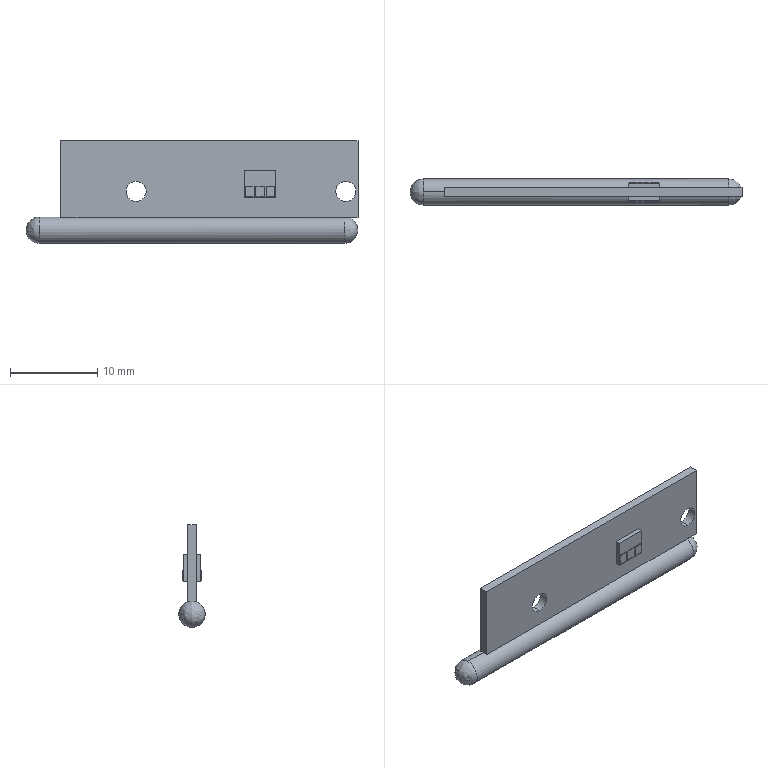Part | SolidWorks | features BaseBody 1 | 1 solid | 54 faces | box 37.94 x 3 x 11.75 mm | volume 563.627 mm3 | plane 46 | cylinder 6 | spline 2 | commonest cylinder face diameters 2.3 x4 3 x2
STEP:
#1=CARTESIAN_POINT('',(32.5,1.,-3.036));
#2=VERTEX_POINT('',#1);
#3=CARTESIAN_POINT('',(32.5,0.5,-5.95));
#4=VERTEX_POINT('',#3);
#5=CARTESIAN_POINT('',(32.5,0.5,-4.45));
#6=DIRECTION('',(-1.,0.,0.));
#7=DIRECTION('',(0.,0.,1.));
#8=AXIS2_PLACEMENT_3D('',#5,#6,#7);
#9=CIRCLE('',#8,1.5);
#10=EDGE_CURVE('',#2,#4,#9,.T.);
#11=ORIENTED_EDGE('',*,*,#10,.T.);
#12=CARTESIAN_POINT('',(-2.5,0.5,-5.95));
#13=VERTEX_POINT('',#12);
#14=CARTESIAN_POINT('',(0.,0.5,-5.95));
#15=DIRECTION('',(-1.,0.,0.));
#16=VECTOR('',#15,1000.);
#17=LINE('',#14,#16);
#18=EDGE_CURVE('',#4,#13,#17,.T.);
#19=ORIENTED_EDGE('',*,*,#18,.T.);
#20=CARTESIAN_POINT('',(-2.5,0.5,-2.95));
#21=VERTEX_POINT('',#20);
#22=CARTESIAN_POINT('',(-2.5,0.5,-4.45));
#23=DIRECTION('',(1.,0.,0.));
#24=DIRECTION('',(0.,0.,1.));
#25=AXIS2_PLACEMENT_3D('',#22,#23,#24);
#26=CIRCLE('',#25,1.5);
#27=EDGE_CURVE('',#13,#21,#26,.T.);
#28=ORIENTED_EDGE('',*,*,#27,.T.);
#29=CARTESIAN_POINT('',(0.,0.5,-2.95));
#30=VERTEX_POINT('',#29);
#31=CARTESIAN_POINT('',(0.,0.5,-2.95));
#32=DIRECTION('',(-1.,0.,0.));
#33=VECTOR('',#32,1000.);
#34=LINE('',#31,#33);
#35=EDGE_CURVE('',#30,#21,#34,.T.);
#36=ORIENTED_EDGE('',*,*,#35,.F.);
#37=CARTESIAN_POINT('',(0.,1.,-3.036));
#38=VERTEX_POINT('',#37);
#39=CARTESIAN_POINT('',(0.,0.5,-4.45));
#40=DIRECTION('',(1.,0.,0.));
#41=DIRECTION('',(0.,0.,1.));
#42=AXIS2_PLACEMENT_3D('',#39,#40,#41);
#43=CIRCLE('',#42,1.5);
#44=EDGE_CURVE('',#38,#30,#43,.T.);
#45=ORIENTED_EDGE('',*,*,#44,.F.);
#46=CARTESIAN_POINT('',(0.,1.,-3.036));
#47=DIRECTION('',(1.,0.,0.));
#48=VECTOR('',#47,1000.);
#49=LINE('',#46,#48);
#50=EDGE_CURVE('',#38,#2,#49,.T.);
#51=ORIENTED_EDGE('',*,*,#50,.T.);
#52=EDGE_LOOP('',(#11,#19,#28,#36,#45,#51));
#53=FACE_OUTER_BOUND('',#52,.T.);
#54=CARTESIAN_POINT('',(0.,0.5,-4.45));
#55=DIRECTION('',(-1.,0.,0.));
#56=DIRECTION('',(0.,0.,1.));
#57=AXIS2_PLACEMENT_3D('',#54,#55,#56);
#58=CYLINDRICAL_SURFACE('',#57,1.5);
#59=ADVANCED_FACE('',(#53),#58,.T.);
#60=CARTESIAN_POINT('',(8.6,1.,1.15));
#61=VERTEX_POINT('',#60);
#62=CARTESIAN_POINT('',(8.6,1.,-1.15));
#63=VERTEX_POINT('',#62);
#64=CARTESIAN_POINT('',(8.6,1.,0.));
#65=DIRECTION('',(0.,-1.,0.));
#66=DIRECTION('',(0.,0.,-1.));
#67=AXIS2_PLACEMENT_3D('',#64,#65,#66);
#68=CIRCLE('',#67,1.15);
#69=EDGE_CURVE('',#61,#63,#68,.T.);
#70=ORIENTED_EDGE('',*,*,#69,.F.);
#71=CARTESIAN_POINT('',(8.6,0.,1.15));
#72=VERTEX_POINT('',#71);
#73=CARTESIAN_POINT('',(8.6,0.,1.15));
#74=DIRECTION('',(0.,-1.,0.));
#75=VECTOR('',#74,1000.);
#76=LINE('',#73,#75);
#77=EDGE_CURVE('',#61,#72,#76,.T.);
#78=ORIENTED_EDGE('',*,*,#77,.T.);
#79=CARTESIAN_POINT('',(8.6,0.,-1.15));
#80=VERTEX_POINT('',#79);
#81=CARTESIAN_POINT('',(8.6,0.,0.));
#82=DIRECTION('',(0.,-1.,0.));
#83=DIRECTION('',(0.,0.,-1.));
#84=AXIS2_PLACEMENT_3D('',#81,#82,#83);
#85=CIRCLE('',#84,1.15);
#86=EDGE_CURVE('',#72,#80,#85,.T.);
#87=ORIENTED_EDGE('',*,*,#86,.T.);
#88=CARTESIAN_POINT('',(8.6,0.,-1.15));
#89=DIRECTION('',(0.,-1.,0.));
#90=VECTOR('',#89,1000.);
#91=LINE('',#88,#90);
#92=EDGE_CURVE('',#63,#80,#91,.T.);
#93=ORIENTED_EDGE('',*,*,#92,.F.);
#94=EDGE_LOOP('',(#70,#78,#87,#93));
#95=FACE_OUTER_BOUND('',#94,.T.);
#96=CARTESIAN_POINT('',(8.6,0.,0.));
#97=DIRECTION('',(0.,-1.,0.));
#98=DIRECTION('',(0.,0.,-1.));
#99=AXIS2_PLACEMENT_3D('',#96,#97,#98);
#100=CYLINDRICAL_SURFACE('',#99,1.15);
#101=ADVANCED_FACE('',(#95),#100,.F.);
#102=CARTESIAN_POINT('',(32.6,1.,1.15));
#103=VERTEX_POINT('',#102);
#104=CARTESIAN_POINT('',(32.6,1.,-1.15));
#105=VERTEX_POINT('',#104);
#106=CARTESIAN_POINT('',(32.6,1.,0.));
#107=DIRECTION('',(0.,-1.,0.));
#108=DIRECTION('',(0.,0.,-1.));
#109=AXIS2_PLACEMENT_3D('',#106,#107,#108);
#110=CIRCLE('',#109,1.15);
#111=EDGE_CURVE('',#103,#105,#110,.T.);
#112=ORIENTED_EDGE('',*,*,#111,.F.);
#113=CARTESIAN_POINT('',(32.6,0.,1.15));
#114=VERTEX_POINT('',#113);
#115=CARTESIAN_POINT('',(32.6,0.,1.15));
#116=DIRECTION('',(0.,-1.,0.));
#117=VECTOR('',#116,1000.);
#118=LINE('',#115,#117);
#119=EDGE_CURVE('',#103,#114,#118,.T.);
#120=ORIENTED_EDGE('',*,*,#119,.T.);
#121=CARTESIAN_POINT('',(32.6,0.,-1.15));
#122=VERTEX_POINT('',#121);
#123=CARTESIAN_POINT('',(32.6,0.,0.));
#124=DIRECTION('',(0.,-1.,0.));
#125=DIRECTION('',(0.,0.,-1.));
#126=AXIS2_PLACEMENT_3D('',#123,#124,#125);
#127=CIRCLE('',#126,1.15);
#128=EDGE_CURVE('',#114,#122,#127,.T.);
#129=ORIENTED_EDGE('',*,*,#128,.T.);
#130=CARTESIAN_POINT('',(32.6,0.,-1.15));
#131=DIRECTION('',(0.,-1.,0.));
#132=VECTOR('',#131,1000.);
#133=LINE('',#130,#132);
#134=EDGE_CURVE('',#105,#122,#133,.T.);
#135=ORIENTED_EDGE('',*,*,#134,.F.);
#136=EDGE_LOOP('',(#112,#120,#129,#135));
#137=FACE_OUTER_BOUND('',#136,.T.);
#138=CARTESIAN_POINT('',(32.6,0.,0.));
#139=DIRECTION('',(0.,-1.,0.));
#140=DIRECTION('',(0.,0.,-1.));
#141=AXIS2_PLACEMENT_3D('',#138,#139,#140);
#142=CYLINDRICAL_SURFACE('',#141,1.15);
#143=ADVANCED_FACE('',(#137),#142,.F.);
#144=ORIENTED_EDGE('',*,*,#18,.F.);
#145=CARTESIAN_POINT('',(32.5,0.,-3.036));
#146=VERTEX_POINT('',#145);
#147=CARTESIAN_POINT('',(32.5,0.5,-4.45));
#148=DIRECTION('',(-1.,0.,0.));
#149=DIRECTION('',(0.,0.,1.));
#150=AXIS2_PLACEMENT_3D('',#147,#148,#149);
#151=CIRCLE('',#150,1.5);
#152=EDGE_CURVE('',#4,#146,#151,.T.);
#153=ORIENTED_EDGE('',*,*,#152,.T.);
#154=CARTESIAN_POINT('',(0.,0.,-3.036));
#155=VERTEX_POINT('',#154);
#156=CARTESIAN_POINT('',(0.,0.,-3.036));
#157=DIRECTION('',(-1.,0.,0.));
#158=VECTOR('',#157,1000.);
#159=LINE('',#156,#158);
#160=EDGE_CURVE('',#146,#155,#159,.T.);
#161=ORIENTED_EDGE('',*,*,#160,.T.);
#162=CARTESIAN_POINT('',(0.,0.5,-4.45));
#163=DIRECTION('',(1.,0.,0.));
#164=DIRECTION('',(0.,0.,1.));
#165=AXIS2_PLACEMENT_3D('',#162,#163,#164);
#166=CIRCLE('',#165,1.5);
#167=EDGE_CURVE('',#30,#155,#166,.T.);
#168=ORIENTED_EDGE('',*,*,#167,.F.);
#169=ORIENTED_EDGE('',*,*,#35,.T.);
#170=CARTESIAN_POINT('',(-2.5,0.5,-4.45));
#171=DIRECTION('',(1.,0.,0.));
#172=DIRECTION('',(0.,0.,1.));
#173=AXIS2_PLACEMENT_3D('',#170,#171,#172);
#174=CIRCLE('',#173,1.5);
#175=EDGE_CURVE('',#21,#13,#174,.T.);
#176=ORIENTED_EDGE('',*,*,#175,.T.);
#177=EDGE_LOOP('',(#144,#153,#161,#168,#169,#176));
#178=FACE_OUTER_BOUND('',#177,.T.);
#179=CARTESIAN_POINT('',(0.,0.5,-4.45));
#180=DIRECTION('',(-1.,0.,0.));
#181=DIRECTION('',(0.,0.,1.));
#182=AXIS2_PLACEMENT_3D('',#179,#180,#181);
#183=CYLINDRICAL_SURFACE('',#182,1.5);
#184=ADVANCED_FACE('',(#178),#183,.T.);
#185=ORIENTED_EDGE('',*,*,#175,.F.);
#186=ORIENTED_EDGE('',*,*,#27,.F.);
#187=EDGE_LOOP('',(#185,#186));
#188=FACE_OUTER_BOUND('',#187,.T.);
#189=CARTESIAN_POINT('',(-2.5,0.5,-5.95));
#190=CARTESIAN_POINT('',(-2.5,0.5,-5.95));
#191=CARTESIAN_POINT('',(-2.5,0.5,-5.95));
#192=CARTESIAN_POINT('',(-2.5,0.5,-5.95));
#193=CARTESIAN_POINT('',(-2.5,-2.5,-5.95));
#194=CARTESIAN_POINT('',(-8.5,-2.5,-5.95));
#195=CARTESIAN_POINT('',(-8.5,3.5,-5.95));
#196=CARTESIAN_POINT('',(-2.5,3.5,-5.95));
#197=CARTESIAN_POINT('',(-2.5,-2.5,-2.95));
#198=CARTESIAN_POINT('',(-8.5,-2.5,-2.95));
#199=CARTESIAN_POINT('',(-8.5,3.5,-2.95));
#200=CARTESIAN_POINT('',(-2.5,3.5,-2.95));
#201=CARTESIAN_POINT('',(-2.5,0.5,-2.95));
#202=CARTESIAN_POINT('',(-2.5,0.5,-2.95));
#203=CARTESIAN_POINT('',(-2.5,0.5,-2.95));
#204=CARTESIAN_POINT('',(-2.5,0.5,-2.95));
#205=(BOUNDED_SURFACE()B_SPLINE_SURFACE(3,3,((#189,#190,#191,#192),(#193,#194,#195,#196),(#197,#198,#199,#200),(#201,#202,#203,#204)),.UNSPECIFIED.,.F.,.F.,.F.)B_SPLINE_SURFACE_WITH_KNOTS((4,4),(4,4),(0.,1.),(0.,1.),.UNSPECIFIED.)GEOMETRIC_REPRESENTATION_ITEM()RATIONAL_B_SPLINE_SURFACE(((1.,0.3333,0.3333,1.),(0.3333,0.1111,0.1111,0.3333),(0.3333,0.1111,0.1111,0.3333),(1.,0.3333,0.3333,1.)))REPRESENTATION_ITEM('')SURFACE());
#206=ADVANCED_FACE('',(#188),#205,.T.);
#207=CARTESIAN_POINT('',(24.6,0.,-0.75));
#208=VERTEX_POINT('',#207);
#209=CARTESIAN_POINT('',(24.6,0.,2.35));
#210=VERTEX_POINT('',#209);
#211=CARTESIAN_POINT('',(24.6,0.,0.));
#212=DIRECTION('',(0.,0.,1.));
#213=VECTOR('',#212,1000.);
#214=LINE('',#211,#213);
#215=EDGE_CURVE('',#208,#210,#214,.T.);
#216=ORIENTED_EDGE('',*,*,#215,.F.);
#217=CARTESIAN_POINT('',(21.,0.,-0.75));
#218=VERTEX_POINT('',#217);
#219=CARTESIAN_POINT('',(0.,0.,-0.75));
#220=DIRECTION('',(1.,0.,0.));
#221=VECTOR('',#220,1000.);
#222=LINE('',#219,#221);
#223=EDGE_CURVE('',#218,#208,#222,.T.);
#224=ORIENTED_EDGE('',*,*,#223,.F.);
#225=CARTESIAN_POINT('',(21.,0.,2.35));
#226=VERTEX_POINT('',#225);
#227=CARTESIAN_POINT('',(21.,0.,0.));
#228=DIRECTION('',(0.,0.,-1.));
#229=VECTOR('',#228,1000.);
#230=LINE('',#227,#229);
#231=EDGE_CURVE('',#226,#218,#230,.T.);
#232=ORIENTED_EDGE('',*,*,#231,.F.);
#233=CARTESIAN_POINT('',(0.,0.,2.35));
#234=DIRECTION('',(-1.,0.,0.));
#235=VECTOR('',#234,1000.);
#236=LINE('',#233,#235);
#237=EDGE_CURVE('',#210,#226,#236,.T.);
#238=ORIENTED_EDGE('',*,*,#237,.F.);
#239=EDGE_LOOP('',(#216,#224,#232,#238));
#240=FACE_BOUND('',#239,.T.);
#241=CARTESIAN_POINT('',(8.6,0.,0.));
#242=DIRECTION('',(0.,-1.,0.));
#243=DIRECTION('',(0.,0.,-1.));
#244=AXIS2_PLACEMENT_3D('',#241,#242,#243);
#245=CIRCLE('',#244,1.15);
#246=EDGE_CURVE('',#80,#72,#245,.T.);
#247=ORIENTED_EDGE('',*,*,#246,.F.);
#248=ORIENTED_EDGE('',*,*,#86,.F.);
#249=EDGE_LOOP('',(#247,#248));
#250=FACE_BOUND('',#249,.T.);
#251=CARTESIAN_POINT('',(32.6,0.,0.));
#252=DIRECTION('',(0.,-1.,0.));
#253=DIRECTION('',(0.,0.,-1.));
#254=AXIS2_PLACEMENT_3D('',#251,#252,#253);
#255=CIRCLE('',#254,1.15);
#256=EDGE_CURVE('',#122,#114,#255,.T.);
#257=ORIENTED_EDGE('',*,*,#256,.F.);
#258=ORIENTED_EDGE('',*,*,#128,.F.);
#259=EDGE_LOOP('',(#257,#258));
#260=FACE_BOUND('',#259,.T.);
#261=CARTESIAN_POINT('',(34.,0.,-3.036));
#262=VERTEX_POINT('',#261);
#263=CARTESIAN_POINT('',(0.,0.,-3.036));
#264=DIRECTION('',(-1.,0.,0.));
#265=VECTOR('',#264,1000.);
#266=LINE('',#263,#265);
#267=EDGE_CURVE('',#262,#146,#266,.T.);
#268=ORIENTED_EDGE('',*,*,#267,.F.);
#269=CARTESIAN_POINT('',(34.,0.,5.8));
#270=VERTEX_POINT('',#269);
#271=CARTESIAN_POINT('',(34.,0.,0.));
#272=DIRECTION('',(0.,0.,-1.));
#273=VECTOR('',#272,1000.);
#274=LINE('',#271,#273);
#275=EDGE_CURVE('',#270,#262,#274,.T.);
#276=ORIENTED_EDGE('',*,*,#275,.F.);
#277=CARTESIAN_POINT('',(0.,0.,5.8));
#278=VERTEX_POINT('',#277);
#279=CARTESIAN_POINT('',(0.,0.,5.8));
#280=DIRECTION('',(1.,0.,0.));
#281=VECTOR('',#280,1000.);
#282=LINE('',#279,#281);
#283=EDGE_CURVE('',#278,#270,#282,.T.);
#284=ORIENTED_EDGE('',*,*,#283,.F.);
#285=CARTESIAN_POINT('',(0.,0.,0.));
#286=DIRECTION('',(0.,0.,1.));
#287=VECTOR('',#286,1000.);
#288=LINE('',#285,#287);
#289=EDGE_CURVE('',#155,#278,#288,.T.);
#290=ORIENTED_EDGE('',*,*,#289,.F.);
#291=ORIENTED_EDGE('',*,*,#160,.F.);
#292=EDGE_LOOP('',(#268,#276,#284,#290,#291));
#293=FACE_OUTER_BOUND('',#292,.T.);
#294=CARTESIAN_POINT('',(0.,0.,0.));
#295=DIRECTION('',(0.,1.,0.));
#296=DIRECTION('',(0.,0.,1.));
#297=AXIS2_PLACEMENT_3D('',#294,#295,#296);
#298=PLANE('',#297);
#299=ADVANCED_FACE('',(#240,#250,#260,#293),#298,.F.);
#300=CARTESIAN_POINT('',(32.5,0.5,-3.036));
#301=DIRECTION('',(0.,0.,-1.));
#302=DIRECTION('',(-1.,0.,0.));
#303=AXIS2_PLACEMENT_3D('',#300,#301,#302);
#304=CIRCLE('',#303,0.5);
#305=EDGE_CURVE('',#2,#146,#304,.T.);
#306=ORIENTED_EDGE('',*,*,#305,.T.);
#307=ORIENTED_EDGE('',*,*,#152,.F.);
#308=ORIENTED_EDGE('',*,*,#10,.F.);
#309=EDGE_LOOP('',(#306,#307,#308));
#310=FACE_OUTER_BOUND('',#309,.T.);
#311=CARTESIAN_POINT('',(32.5,0.5,-5.95));
#312=CARTESIAN_POINT('',(32.5,0.5,-5.95));
#313=CARTESIAN_POINT('',(32.5,0.5,-5.95));
#314=CARTESIAN_POINT('',(32.5,0.5,-5.95));
#315=CARTESIAN_POINT('',(32.5,2.71,-5.95));
#316=CARTESIAN_POINT('',(36.919,2.71,-5.95));
#317=CARTESIAN_POINT('',(36.919,-1.71,-5.95));
#318=CARTESIAN_POINT('',(32.5,-1.71,-5.95));
#319=CARTESIAN_POINT('',(32.5,3.083,-3.772));
#320=CARTESIAN_POINT('',(37.666,3.083,-3.772));
#321=CARTESIAN_POINT('',(37.666,-2.083,-3.772));
#322=CARTESIAN_POINT('',(32.5,-2.083,-3.772));
#323=CARTESIAN_POINT('',(32.5,1.,-3.036));
#324=CARTESIAN_POINT('',(33.5,1.,-3.036));
#325=CARTESIAN_POINT('',(33.5,0.,-3.036));
#326=CARTESIAN_POINT('',(32.5,0.,-3.036));
#327=(BOUNDED_SURFACE()B_SPLINE_SURFACE(3,3,((#311,#312,#313,#314),(#315,#316,#317,#318),(#319,#320,#321,#322),(#323,#324,#325,#326)),.UNSPECIFIED.,.F.,.F.,.F.)B_SPLINE_SURFACE_WITH_KNOTS((4,4),(4,4),(0.,1.),(0.,1.),.UNSPECIFIED.)GEOMETRIC_REPRESENTATION_ITEM()RATIONAL_B_SPLINE_SURFACE(((1.,0.3333,0.3333,1.),(0.4461,0.1487,0.1487,0.4461),(0.4461,0.1487,0.1487,0.4461),(1.,0.3333,0.3333,1.)))REPRESENTATION_ITEM('')SURFACE());
#328=ADVANCED_FACE('',(#310),#327,.T.);
#329=CARTESIAN_POINT('',(24.6,1.,2.35));
#330=VERTEX_POINT('',#329);
#331=CARTESIAN_POINT('',(21.,1.,2.35));
#332=VERTEX_POINT('',#331);
#333=CARTESIAN_POINT('',(0.,1.,2.35));
#334=DIRECTION('',(-1.,0.,0.));
#335=VECTOR('',#334,1000.);
#336=LINE('',#333,#335);
#337=EDGE_CURVE('',#330,#332,#336,.T.);
#338=ORIENTED_EDGE('',*,*,#337,.T.);
#339=CARTESIAN_POINT('',(21.,1.,-0.75));
#340=VERTEX_POINT('',#339);
#341=CARTESIAN_POINT('',(21.,1.,0.));
#342=DIRECTION('',(0.,0.,-1.));
#343=VECTOR('',#342,1000.);
#344=LINE('',#341,#343);
#345=EDGE_CURVE('',#332,#340,#344,.T.);
#346=ORIENTED_EDGE('',*,*,#345,.T.);
#347=CARTESIAN_POINT('',(24.6,1.,-0.75));
#348=VERTEX_POINT('',#347);
#349=CARTESIAN_POINT('',(0.,1.,-0.75));
#350=DIRECTION('',(1.,0.,0.));
#351=VECTOR('',#350,1000.);
#352=LINE('',#349,#351);
#353=EDGE_CURVE('',#340,#348,#352,.T.);
#354=ORIENTED_EDGE('',*,*,#353,.T.);
#355=CARTESIAN_POINT('',(24.6,1.,0.));
#356=DIRECTION('',(0.,0.,1.));
#357=VECTOR('',#356,1000.);
#358=LINE('',#355,#357);
#359=EDGE_CURVE('',#348,#330,#358,.T.);
#360=ORIENTED_EDGE('',*,*,#359,.T.);
#361=EDGE_LOOP('',(#338,#346,#354,#360));
#362=FACE_BOUND('',#361,.T.);
#363=CARTESIAN_POINT('',(8.6,1.,0.));
#364=DIRECTION('',(0.,-1.,0.));
#365=DIRECTION('',(0.,0.,-1.));
#366=AXIS2_PLACEMENT_3D('',#363,#364,#365);
#367=CIRCLE('',#366,1.15);
#368=EDGE_CURVE('',#63,#61,#367,.T.);
#369=ORIENTED_EDGE('',*,*,#368,.T.);
#370=ORIENTED_EDGE('',*,*,#69,.T.);
#371=EDGE_LOOP('',(#369,#370));
#372=FACE_BOUND('',#371,.T.);
#373=CARTESIAN_POINT('',(32.6,1.,0.));
#374=DIRECTION('',(0.,-1.,0.));
#375=DIRECTION('',(0.,0.,-1.));
#376=AXIS2_PLACEMENT_3D('',#373,#374,#375);
#377=CIRCLE('',#376,1.15);
#378=EDGE_CURVE('',#105,#103,#377,.T.);
#379=ORIENTED_EDGE('',*,*,#378,.T.);
#380=ORIENTED_EDGE('',*,*,#111,.T.);
#381=EDGE_LOOP('',(#379,#380));
#382=FACE_BOUND('',#381,.T.);
#383=ORIENTED_EDGE('',*,*,#50,.F.);
#384=CARTESIAN_POINT('',(0.,1.,5.8));
#385=VERTEX_POINT('',#384);
#386=CARTESIAN_POINT('',(0.,1.,0.));
#387=DIRECTION('',(0.,0.,1.));
#388=VECTOR('',#387,1000.);
#389=LINE('',#386,#388);
#390=EDGE_CURVE('',#38,#385,#389,.T.);
#391=ORIENTED_EDGE('',*,*,#390,.T.);
#392=CARTESIAN_POINT('',(34.,1.,5.8));
#393=VERTEX_POINT('',#392);
#394=CARTESIAN_POINT('',(0.,1.,5.8));
#395=DIRECTION('',(1.,0.,0.));
#396=VECTOR('',#395,1000.);
#397=LINE('',#394,#396);
#398=EDGE_CURVE('',#385,#393,#397,.T.);
#399=ORIENTED_EDGE('',*,*,#398,.T.);
#400=CARTESIAN_POINT('',(34.,1.,-3.036));
#401=VERTEX_POINT('',#400);
#402=CARTESIAN_POINT('',(34.,1.,0.));
#403=DIRECTION('',(0.,0.,-1.));
#404=VECTOR('',#403,1000.);
#405=LINE('',#402,#404);
#406=EDGE_CURVE('',#393,#401,#405,.T.);
#407=ORIENTED_EDGE('',*,*,#406,.T.);
#408=CARTESIAN_POINT('',(0.,1.,-3.036));
#409=DIRECTION('',(-1.,0.,0.));
#410=VECTOR('',#409,1000.);
#411=LINE('',#408,#410);
#412=EDGE_CURVE('',#401,#2,#411,.T.);
#413=ORIENTED_EDGE('',*,*,#412,.T.);
#414=EDGE_LOOP('',(#383,#391,#399,#407,#413));
#415=FACE_OUTER_BOUND('',#414,.T.);
#416=CARTESIAN_POINT('',(0.,1.,0.));
#417=DIRECTION('',(0.,1.,0.));
#418=DIRECTION('',(0.,0.,1.));
#419=AXIS2_PLACEMENT_3D('',#416,#417,#418);
#420=PLANE('',#419);
#421=ADVANCED_FACE('',(#362,#372,#382,#415),#420,.T.);
#422=CARTESIAN_POINT('',(24.6,-0.5,2.35));
#423=VERTEX_POINT('',#422);
#424=CARTESIAN_POINT('',(24.6,0.,2.35));
#425=DIRECTION('',(0.,1.,0.));
#426=VECTOR('',#425,1000.);
#427=LINE('',#424,#426);
#428=EDGE_CURVE('',#423,#210,#427,.T.);
#429=ORIENTED_EDGE('',*,*,#428,.T.);
#430=ORIENTED_EDGE('',*,*,#237,.T.);
#431=CARTESIAN_POINT('',(21.,-0.5,2.35));
#432=VERTEX_POINT('',#431);
#433=CARTESIAN_POINT('',(21.,0.,2.35));
#434=DIRECTION('',(0.,-1.,0.));
#435=VECTOR('',#434,1000.);
#436=LINE('',#433,#435);
#437=EDGE_CURVE('',#226,#432,#436,.T.);
#438=ORIENTED_EDGE('',*,*,#437,.T.);
#439=CARTESIAN_POINT('',(24.6,-0.5,2.35));
#440=DIRECTION('',(1.,0.,0.));
#441=VECTOR('',#440,1000.);
#442=LINE('',#439,#441);
#443=EDGE_CURVE('',#432,#423,#442,.T.);
#444=ORIENTED_EDGE('',*,*,#443,.T.);
#445=EDGE_LOOP('',(#429,#430,#438,#444));
#446=FACE_OUTER_BOUND('',#445,.T.);
#447=CARTESIAN_POINT('',(24.6,0.,2.35));
#448=DIRECTION('',(0.,0.,1.));
#449=DIRECTION('',(1.,0.,0.));
#450=AXIS2_PLACEMENT_3D('',#447,#448,#449);
#451=PLANE('',#450);
#452=ADVANCED_FACE('',(#446),#451,.T.);
#453=CARTESIAN_POINT('',(24.6,-0.5,-0.75));
#454=VERTEX_POINT('',#453);
#455=CARTESIAN_POINT('',(24.6,0.,-0.75));
#456=DIRECTION('',(0.,1.,0.));
#457=VECTOR('',#456,1000.);
#458=LINE('',#455,#457);
#459=EDGE_CURVE('',#454,#208,#458,.T.);
#460=ORIENTED_EDGE('',*,*,#459,.T.);
#461=ORIENTED_EDGE('',*,*,#215,.T.);
#462=ORIENTED_EDGE('',*,*,#428,.F.);
#463=CARTESIAN_POINT('',(24.6,-0.5,-0.75));
#464=DIRECTION('',(0.,0.,-1.));
#465=VECTOR('',#464,1000.);
#466=LINE('',#463,#465);
#467=EDGE_CURVE('',#423,#454,#466,.T.);
#468=ORIENTED_EDGE('',*,*,#467,.T.);
#469=EDGE_LOOP('',(#460,#461,#462,#468));
#470=FACE_OUTER_BOUND('',#469,.T.);
#471=CARTESIAN_POINT('',(24.6,0.,-0.75));
#472=DIRECTION('',(1.,0.,0.));
#473=DIRECTION('',(0.,0.,-1.));
#474=AXIS2_PLACEMENT_3D('',#471,#472,#473);
#475=PLANE('',#474);
#476=ADVANCED_FACE('',(#470),#475,.T.);
#477=CARTESIAN_POINT('',(21.,-0.5,-0.75));
#478=VERTEX_POINT('',#477);
#479=CARTESIAN_POINT('',(21.,0.,-0.75));
#480=DIRECTION('',(0.,1.,0.));
#481=VECTOR('',#480,1000.);
#482=LINE('',#479,#481);
#483=EDGE_CURVE('',#478,#218,#482,.T.);
#484=ORIENTED_EDGE('',*,*,#483,.T.);
#485=ORIENTED_EDGE('',*,*,#223,.T.);
#486=ORIENTED_EDGE('',*,*,#459,.F.);
#487=CARTESIAN_POINT('',(21.,-0.5,-0.75));
#488=DIRECTION('',(-1.,0.,0.));
#489=VECTOR('',#488,1000.);
#490=LINE('',#487,#489);
#491=EDGE_CURVE('',#454,#478,#490,.T.);
#492=ORIENTED_EDGE('',*,*,#491,.T.);
#493=EDGE_LOOP('',(#484,#485,#486,#492));
#494=FACE_OUTER_BOUND('',#493,.T.);
#495=CARTESIAN_POINT('',(21.,0.,-0.75));
#496=DIRECTION('',(0.,0.,-1.));
#497=DIRECTION('',(-1.,0.,0.));
#498=AXIS2_PLACEMENT_3D('',#495,#496,#497);
#499=PLANE('',#498);
#500=ADVANCED_FACE('',(#494),#499,.T.);
#501=ORIENTED_EDGE('',*,*,#437,.F.);
#502=ORIENTED_EDGE('',*,*,#231,.T.);
#503=ORIENTED_EDGE('',*,*,#483,.F.);
#504=CARTESIAN_POINT('',(21.,-0.5,2.35));
#505=DIRECTION('',(0.,0.,1.));
#506=VECTOR('',#505,1000.);
#507=LINE('',#504,#506);
#508=EDGE_CURVE('',#478,#432,#507,.T.);
#509=ORIENTED_EDGE('',*,*,#508,.T.);
#510=EDGE_LOOP('',(#501,#502,#503,#509));
#511=FACE_OUTER_BOUND('',#510,.T.);
#512=CARTESIAN_POINT('',(21.,0.,2.35));
#513=DIRECTION('',(-1.,0.,0.));
#514=DIRECTION('',(0.,0.,1.));
#515=AXIS2_PLACEMENT_3D('',#512,#513,#514);
#516=PLANE('',#515);
#517=ADVANCED_FACE('',(#511),#516,.T.);
#518=ORIENTED_EDGE('',*,*,#77,.F.);
#519=ORIENTED_EDGE('',*,*,#368,.F.);
#520=ORIENTED_EDGE('',*,*,#92,.T.);
#521=ORIENTED_EDGE('',*,*,#246,.T.);
#522=EDGE_LOOP('',(#518,#519,#520,#521));
#523=FACE_OUTER_BOUND('',#522,.T.);
#524=CARTESIAN_POINT('',(8.6,0.,0.));
#525=DIRECTION('',(0.,-1.,0.));
#526=DIRECTION('',(0.,0.,-1.));
#527=AXIS2_PLACEMENT_3D('',#524,#525,#526);
#528=CYLINDRICAL_SURFACE('',#527,1.15);
#529=ADVANCED_FACE('',(#523),#528,.F.);
#530=ORIENTED_EDGE('',*,*,#119,.F.);
#531=ORIENTED_EDGE('',*,*,#378,.F.);
#532=ORIENTED_EDGE('',*,*,#134,.T.);
#533=ORIENTED_EDGE('',*,*,#256,.T.);
#534=EDGE_LOOP('',(#530,#531,#532,#533));
#535=FACE_OUTER_BOUND('',#534,.T.);
#536=CARTESIAN_POINT('',(32.6,0.,0.));
#537=DIRECTION('',(0.,-1.,0.));
#538=DIRECTION('',(0.,0.,-1.));
#539=AXIS2_PLACEMENT_3D('',#536,#537,#538);
#540=CYLINDRICAL_SURFACE('',#539,1.15);
#541=ADVANCED_FACE('',(#535),#540,.F.);
#542=ORIENTED_EDGE('',*,*,#412,.F.);
#543=CARTESIAN_POINT('',(34.,-4.51,-3.036));
#544=DIRECTION('',(0.,1.,0.));
#545=VECTOR('',#544,1000.);
#546=LINE('',#543,#545);
#547=EDGE_CURVE('',#262,#401,#546,.T.);
#548=ORIENTED_EDGE('',*,*,#547,.F.);
#549=ORIENTED_EDGE('',*,*,#267,.T.);
#550=ORIENTED_EDGE('',*,*,#305,.F.);
#551=EDGE_LOOP('',(#542,#548,#549,#550));
#552=FACE_OUTER_BOUND('',#551,.T.);
#553=CARTESIAN_POINT('',(35.721,-4.51,-3.036));
#554=DIRECTION('',(0.,0.,1.));
#555=DIRECTION('',(1.,0.,0.));
#556=AXIS2_PLACEMENT_3D('',#553,#554,#555);
#557=PLANE('',#556);
#558=ADVANCED_FACE('',(#552),#557,.F.);
#559=CARTESIAN_POINT('',(34.,0.,5.8));
#560=DIRECTION('',(0.,-1.,0.));
#561=VECTOR('',#560,1000.);
#562=LINE('',#559,#561);
#563=EDGE_CURVE('',#393,#270,#562,.T.);
#564=ORIENTED_EDGE('',*,*,#563,.T.);
#565=ORIENTED_EDGE('',*,*,#275,.T.);
#566=ORIENTED_EDGE('',*,*,#547,.T.);
#567=ORIENTED_EDGE('',*,*,#406,.F.);
#568=EDGE_LOOP('',(#564,#565,#566,#567));
#569=FACE_OUTER_BOUND('',#568,.T.);
#570=CARTESIAN_POINT('',(34.,0.,5.8));
#571=DIRECTION('',(1.,0.,0.));
#572=DIRECTION('',(0.,0.,-1.));
#573=AXIS2_PLACEMENT_3D('',#570,#571,#572);
#574=PLANE('',#573);
#575=ADVANCED_FACE('',(#569),#574,.T.);
#576=ORIENTED_EDGE('',*,*,#563,.F.);
#577=ORIENTED_EDGE('',*,*,#398,.F.);
#578=CARTESIAN_POINT('',(0.,0.,5.8));
#579=DIRECTION('',(0.,-1.,0.));
#580=VECTOR('',#579,1000.);
#581=LINE('',#578,#580);
#582=EDGE_CURVE('',#385,#278,#581,.T.);
#583=ORIENTED_EDGE('',*,*,#582,.T.);
#584=ORIENTED_EDGE('',*,*,#283,.T.);
#585=EDGE_LOOP('',(#576,#577,#583,#584));
#586=FACE_OUTER_BOUND('',#585,.T.);
#587=CARTESIAN_POINT('',(0.,0.,5.8));
#588=DIRECTION('',(0.,0.,1.));
#589=DIRECTION('',(1.,0.,0.));
#590=AXIS2_PLACEMENT_3D('',#587,#588,#589);
#591=PLANE('',#590);
#592=ADVANCED_FACE('',(#586),#591,.T.);
#593=ORIENTED_EDGE('',*,*,#582,.F.);
#594=ORIENTED_EDGE('',*,*,#390,.F.);
#595=ORIENTED_EDGE('',*,*,#44,.T.);
#596=ORIENTED_EDGE('',*,*,#167,.T.);
#597=ORIENTED_EDGE('',*,*,#289,.T.);
#598=EDGE_LOOP('',(#593,#594,#595,#596,#597));
#599=FACE_OUTER_BOUND('',#598,.T.);
#600=CARTESIAN_POINT('',(0.,0.,-5.8));
#601=DIRECTION('',(-1.,0.,0.));
#602=DIRECTION('',(0.,0.,1.));
#603=AXIS2_PLACEMENT_3D('',#600,#601,#602);
#604=PLANE('',#603);
#605=ADVANCED_FACE('',(#599),#604,.T.);
#606=CARTESIAN_POINT('',(21.,1.5,-0.75));
#607=VERTEX_POINT('',#606);
#608=CARTESIAN_POINT('',(21.,1.5,2.35));
#609=VERTEX_POINT('',#608);
#610=CARTESIAN_POINT('',(21.,1.5,2.35));
#611=DIRECTION('',(0.,0.,1.));
#612=VECTOR('',#611,1000.);
#613=LINE('',#610,#612);
#614=EDGE_CURVE('',#607,#609,#613,.T.);
#615=ORIENTED_EDGE('',*,*,#614,.F.);
#616=CARTESIAN_POINT('',(21.,1.,-0.75));
#617=DIRECTION('',(0.,1.,0.));
#618=VECTOR('',#617,1000.);
#619=LINE('',#616,#618);
#620=EDGE_CURVE('',#340,#607,#619,.T.);
#621=ORIENTED_EDGE('',*,*,#620,.F.);
#622=ORIENTED_EDGE('',*,*,#345,.F.);
#623=CARTESIAN_POINT('',(21.,1.,2.35));
#624=DIRECTION('',(0.,-1.,0.));
#625=VECTOR('',#624,1000.);
#626=LINE('',#623,#625);
#627=EDGE_CURVE('',#609,#332,#626,.T.);
#628=ORIENTED_EDGE('',*,*,#627,.F.);
#629=EDGE_LOOP('',(#615,#621,#622,#628));
#630=FACE_OUTER_BOUND('',#629,.T.);
#631=CARTESIAN_POINT('',(21.,1.,2.35));
#632=DIRECTION('',(1.,0.,0.));
#633=DIRECTION('',(0.,0.,-1.));
#634=AXIS2_PLACEMENT_3D('',#631,#632,#633);
#635=PLANE('',#634);
#636=ADVANCED_FACE('',(#630),#635,.F.);
#637=CARTESIAN_POINT('',(24.6,1.5,2.35));
#638=VERTEX_POINT('',#637);
#639=CARTESIAN_POINT('',(24.6,1.5,2.35));
#640=DIRECTION('',(1.,0.,0.));
#641=VECTOR('',#640,1000.);
#642=LINE('',#639,#641);
#643=EDGE_CURVE('',#609,#638,#642,.T.);
#644=ORIENTED_EDGE('',*,*,#643,.F.);
#645=ORIENTED_EDGE('',*,*,#627,.T.);
#646=ORIENTED_EDGE('',*,*,#337,.F.);
#647=CARTESIAN_POINT('',(24.6,1.,2.35));
#648=DIRECTION('',(0.,-1.,0.));
#649=VECTOR('',#648,1000.);
#650=LINE('',#647,#649);
#651=EDGE_CURVE('',#638,#330,#650,.T.);
#652=ORIENTED_EDGE('',*,*,#651,.F.);
#653=EDGE_LOOP('',(#644,#645,#646,#652));
#654=FACE_OUTER_BOUND('',#653,.T.);
#655=CARTESIAN_POINT('',(24.6,1.,2.35));
#656=DIRECTION('',(0.,0.,-1.));
#657=DIRECTION('',(-1.,0.,0.));
#658=AXIS2_PLACEMENT_3D('',#655,#656,#657);
#659=PLANE('',#658);
#660=ADVANCED_FACE('',(#654),#659,.F.);
#661=CARTESIAN_POINT('',(24.6,1.5,-0.75));
#662=VERTEX_POINT('',#661);
#663=CARTESIAN_POINT('',(24.6,1.5,-0.75));
#664=DIRECTION('',(0.,0.,-1.));
#665=VECTOR('',#664,1000.);
#666=LINE('',#663,#665);
#667=EDGE_CURVE('',#638,#662,#666,.T.);
#668=ORIENTED_EDGE('',*,*,#667,.F.);
#669=ORIENTED_EDGE('',*,*,#651,.T.);
#670=ORIENTED_EDGE('',*,*,#359,.F.);
#671=CARTESIAN_POINT('',(24.6,1.,-0.75));
#672=DIRECTION('',(0.,-1.,0.));
#673=VECTOR('',#672,1000.);
#674=LINE('',#671,#673);
#675=EDGE_CURVE('',#662,#348,#674,.T.);
#676=ORIENTED_EDGE('',*,*,#675,.F.);
#677=EDGE_LOOP('',(#668,#669,#670,#676));
#678=FACE_OUTER_BOUND('',#677,.T.);
#679=CARTESIAN_POINT('',(24.6,1.,-0.75));
#680=DIRECTION('',(-1.,0.,0.));
#681=DIRECTION('',(0.,0.,1.));
#682=AXIS2_PLACEMENT_3D('',#679,#680,#681);
#683=PLANE('',#682);
#684=ADVANCED_FACE('',(#678),#683,.F.);
#685=CARTESIAN_POINT('',(21.,1.5,-0.75));
#686=DIRECTION('',(-1.,0.,0.));
#687=VECTOR('',#686,1000.);
#688=LINE('',#685,#687);
#689=EDGE_CURVE('',#662,#607,#688,.T.);
#690=ORIENTED_EDGE('',*,*,#689,.F.);
#691=ORIENTED_EDGE('',*,*,#675,.T.);
#692=ORIENTED_EDGE('',*,*,#353,.F.);
#693=ORIENTED_EDGE('',*,*,#620,.T.);
#694=EDGE_LOOP('',(#690,#691,#692,#693));
#695=FACE_OUTER_BOUND('',#694,.T.);
#696=CARTESIAN_POINT('',(21.,1.,-0.75));
#697=DIRECTION('',(0.,0.,1.));
#698=DIRECTION('',(1.,0.,0.));
#699=AXIS2_PLACEMENT_3D('',#696,#697,#698);
#700=PLANE('',#699);
#701=ADVANCED_FACE('',(#695),#700,.F.);
#702=CARTESIAN_POINT('',(22.1,-0.5,0.6));
#703=VERTEX_POINT('',#702);
#704=CARTESIAN_POINT('',(22.1,-0.5,-0.6));
#705=VERTEX_POINT('',#704);
#706=CARTESIAN_POINT('',(22.1,-0.5,0.));
#707=DIRECTION('',(0.,0.,-1.));
#708=VECTOR('',#707,1000.);
#709=LINE('',#706,#708);
#710=EDGE_CURVE('',#703,#705,#709,.T.);
#711=ORIENTED_EDGE('',*,*,#710,.T.);
#712=CARTESIAN_POINT('',(21.1,-0.5,-0.6));
#713=VERTEX_POINT('',#712);
#714=CARTESIAN_POINT('',(0.,-0.5,-0.6));
#715=DIRECTION('',(-1.,0.,0.));
#716=VECTOR('',#715,1000.);
#717=LINE('',#714,#716);
#718=EDGE_CURVE('',#705,#713,#717,.T.);
#719=ORIENTED_EDGE('',*,*,#718,.T.);
#720=CARTESIAN_POINT('',(21.1,-0.5,0.6));
#721=VERTEX_POINT('',#720);
#722=CARTESIAN_POINT('',(21.1,-0.5,0.));
#723=DIRECTION('',(0.,0.,1.));
#724=VECTOR('',#723,1000.);
#725=LINE('',#722,#724);
#726=EDGE_CURVE('',#713,#721,#725,.T.);
#727=ORIENTED_EDGE('',*,*,#726,.T.);
#728=CARTESIAN_POINT('',(0.,-0.5,0.6));
#729=DIRECTION('',(1.,0.,0.));
#730=VECTOR('',#729,1000.);
#731=LINE('',#728,#730);
#732=EDGE_CURVE('',#721,#703,#731,.T.);
#733=ORIENTED_EDGE('',*,*,#732,.T.);
#734=EDGE_LOOP('',(#711,#719,#727,#733));
#735=FACE_BOUND('',#734,.T.);
#736=CARTESIAN_POINT('',(22.3,-0.5,0.6));
#737=VERTEX_POINT('',#736);
#738=CARTESIAN_POINT('',(23.3,-0.5,0.6));
#739=VERTEX_POINT('',#738);
#740=CARTESIAN_POINT('',(0.,-0.5,0.6));
#741=DIRECTION('',(1.,0.,0.));
#742=VECTOR('',#741,1000.);
#743=LINE('',#740,#742);
#744=EDGE_CURVE('',#737,#739,#743,.T.);
#745=ORIENTED_EDGE('',*,*,#744,.T.);
#746=CARTESIAN_POINT('',(23.3,-0.5,-0.6));
#747=VERTEX_POINT('',#746);
#748=CARTESIAN_POINT('',(23.3,-0.5,0.));
#749=DIRECTION('',(0.,0.,-1.));
#750=VECTOR('',#749,1000.);
#751=LINE('',#748,#750);
#752=EDGE_CURVE('',#739,#747,#751,.T.);
#753=ORIENTED_EDGE('',*,*,#752,.T.);
#754=CARTESIAN_POINT('',(22.3,-0.5,-0.6));
#755=VERTEX_POINT('',#754);
#756=CARTESIAN_POINT('',(0.,-0.5,-0.6));
#757=DIRECTION('',(-1.,0.,0.));
#758=VECTOR('',#757,1000.);
#759=LINE('',#756,#758);
#760=EDGE_CURVE('',#747,#755,#759,.T.);
#761=ORIENTED_EDGE('',*,*,#760,.T.);
#762=CARTESIAN_POINT('',(22.3,-0.5,0.));
#763=DIRECTION('',(0.,0.,1.));
#764=VECTOR('',#763,1000.);
#765=LINE('',#762,#764);
#766=EDGE_CURVE('',#755,#737,#765,.T.);
#767=ORIENTED_EDGE('',*,*,#766,.T.);
#768=EDGE_LOOP('',(#745,#753,#761,#767));
#769=FACE_BOUND('',#768,.T.);
#770=CARTESIAN_POINT('',(23.5,-0.5,0.6));
#771=VERTEX_POINT('',#770);
#772=CARTESIAN_POINT('',(24.5,-0.5,0.6));
#773=VERTEX_POINT('',#772);
#774=CARTESIAN_POINT('',(0.,-0.5,0.6));
#775=DIRECTION('',(1.,0.,0.));
#776=VECTOR('',#775,1000.);
#777=LINE('',#774,#776);
#778=EDGE_CURVE('',#771,#773,#777,.T.);
#779=ORIENTED_EDGE('',*,*,#778,.T.);
#780=CARTESIAN_POINT('',(24.5,-0.5,-0.6));
#781=VERTEX_POINT('',#780);
#782=CARTESIAN_POINT('',(24.5,-0.5,0.));
#783=DIRECTION('',(0.,0.,-1.));
#784=VECTOR('',#783,1000.);
#785=LINE('',#782,#784);
#786=EDGE_CURVE('',#773,#781,#785,.T.);
#787=ORIENTED_EDGE('',*,*,#786,.T.);
#788=CARTESIAN_POINT('',(23.5,-0.5,-0.6));
#789=VERTEX_POINT('',#788);
#790=CARTESIAN_POINT('',(0.,-0.5,-0.6));
#791=DIRECTION('',(-1.,0.,0.));
#792=VECTOR('',#791,1000.);
#793=LINE('',#790,#792);
#794=EDGE_CURVE('',#781,#789,#793,.T.);
#795=ORIENTED_EDGE('',*,*,#794,.T.);
#796=CARTESIAN_POINT('',(23.5,-0.5,0.));
#797=DIRECTION('',(0.,0.,1.));
#798=VECTOR('',#797,1000.);
#799=LINE('',#796,#798);
#800=EDGE_CURVE('',#789,#771,#799,.T.);
#801=ORIENTED_EDGE('',*,*,#800,.T.);
#802=EDGE_LOOP('',(#779,#787,#795,#801));
#803=FACE_BOUND('',#802,.T.);
#804=ORIENTED_EDGE('',*,*,#443,.F.);
#805=ORIENTED_EDGE('',*,*,#508,.F.);
#806=ORIENTED_EDGE('',*,*,#491,.F.);
#807=ORIENTED_EDGE('',*,*,#467,.F.);
#808=EDGE_LOOP('',(#804,#805,#806,#807));
#809=FACE_OUTER_BOUND('',#808,.T.);
#810=CARTESIAN_POINT('',(0.,-0.5,0.));
#811=DIRECTION('',(0.,-1.,0.));
#812=DIRECTION('',(0.,0.,-1.));
#813=AXIS2_PLACEMENT_3D('',#810,#811,#812);
#814=PLANE('',#813);
#815=ADVANCED_FACE('',(#735,#769,#803,#809),#814,.T.);
#816=CARTESIAN_POINT('',(21.1,1.5,0.6));
#817=VERTEX_POINT('',#816);
#818=CARTESIAN_POINT('',(22.1,1.5,0.6));
#819=VERTEX_POINT('',#818);
#820=CARTESIAN_POINT('',(0.,1.5,0.6));
#821=DIRECTION('',(1.,0.,0.));
#822=VECTOR('',#821,1000.);
#823=LINE('',#820,#822);
#824=EDGE_CURVE('',#817,#819,#823,.T.);
#825=ORIENTED_EDGE('',*,*,#824,.F.);
#826=CARTESIAN_POINT('',(21.1,1.5,-0.6));
#827=VERTEX_POINT('',#826);
#828=CARTESIAN_POINT('',(21.1,1.5,0.));
#829=DIRECTION('',(0.,0.,1.));
#830=VECTOR('',#829,1000.);
#831=LINE('',#828,#830);
#832=EDGE_CURVE('',#827,#817,#831,.T.);
#833=ORIENTED_EDGE('',*,*,#832,.F.);
#834=CARTESIAN_POINT('',(22.1,1.5,-0.6));
#835=VERTEX_POINT('',#834);
#836=CARTESIAN_POINT('',(0.,1.5,-0.6));
#837=DIRECTION('',(-1.,0.,0.));
#838=VECTOR('',#837,1000.);
#839=LINE('',#836,#838);
#840=EDGE_CURVE('',#835,#827,#839,.T.);
#841=ORIENTED_EDGE('',*,*,#840,.F.);
#842=CARTESIAN_POINT('',(22.1,1.5,0.));
#843=DIRECTION('',(0.,0.,-1.));
#844=VECTOR('',#843,1000.);
#845=LINE('',#842,#844);
#846=EDGE_CURVE('',#819,#835,#845,.T.);
#847=ORIENTED_EDGE('',*,*,#846,.F.);
#848=EDGE_LOOP('',(#825,#833,#841,#847));
#849=FACE_BOUND('',#848,.T.);
#850=CARTESIAN_POINT('',(22.3,1.5,-0.6));
#851=VERTEX_POINT('',#850);
#852=CARTESIAN_POINT('',(22.3,1.5,0.6));
#853=VERTEX_POINT('',#852);
#854=CARTESIAN_POINT('',(22.3,1.5,0.));
#855=DIRECTION('',(0.,0.,1.));
#856=VECTOR('',#855,1000.);
#857=LINE('',#854,#856);
#858=EDGE_CURVE('',#851,#853,#857,.T.);
#859=ORIENTED_EDGE('',*,*,#858,.F.);
#860=CARTESIAN_POINT('',(23.3,1.5,-0.6));
#861=VERTEX_POINT('',#860);
#862=CARTESIAN_POINT('',(0.,1.5,-0.6));
#863=DIRECTION('',(-1.,0.,0.));
#864=VECTOR('',#863,1000.);
#865=LINE('',#862,#864);
#866=EDGE_CURVE('',#861,#851,#865,.T.);
#867=ORIENTED_EDGE('',*,*,#866,.F.);
#868=CARTESIAN_POINT('',(23.3,1.5,0.6));
#869=VERTEX_POINT('',#868);
#870=CARTESIAN_POINT('',(23.3,1.5,0.));
#871=DIRECTION('',(0.,0.,-1.));
#872=VECTOR('',#871,1000.);
#873=LINE('',#870,#872);
#874=EDGE_CURVE('',#869,#861,#873,.T.);
#875=ORIENTED_EDGE('',*,*,#874,.F.);
#876=CARTESIAN_POINT('',(0.,1.5,0.6));
#877=DIRECTION('',(1.,0.,0.));
#878=VECTOR('',#877,1000.);
#879=LINE('',#876,#878);
#880=EDGE_CURVE('',#853,#869,#879,.T.);
#881=ORIENTED_EDGE('',*,*,#880,.F.);
#882=EDGE_LOOP('',(#859,#867,#875,#881));
#883=FACE_BOUND('',#882,.T.);
#884=CARTESIAN_POINT('',(23.5,1.5,-0.6));
#885=VERTEX_POINT('',#884);
#886=CARTESIAN_POINT('',(23.5,1.5,0.6));
#887=VERTEX_POINT('',#886);
#888=CARTESIAN_POINT('',(23.5,1.5,0.));
#889=DIRECTION('',(0.,0.,1.));
#890=VECTOR('',#889,1000.);
#891=LINE('',#888,#890);
#892=EDGE_CURVE('',#885,#887,#891,.T.);
#893=ORIENTED_EDGE('',*,*,#892,.F.);
#894=CARTESIAN_POINT('',(24.5,1.5,-0.6));
#895=VERTEX_POINT('',#894);
#896=CARTESIAN_POINT('',(0.,1.5,-0.6));
#897=DIRECTION('',(-1.,0.,0.));
#898=VECTOR('',#897,1000.);
#899=LINE('',#896,#898);
#900=EDGE_CURVE('',#895,#885,#899,.T.);
#901=ORIENTED_EDGE('',*,*,#900,.F.);
#902=CARTESIAN_POINT('',(24.5,1.5,0.6));
#903=VERTEX_POINT('',#902);
#904=CARTESIAN_POINT('',(24.5,1.5,0.));
#905=DIRECTION('',(0.,0.,-1.));
#906=VECTOR('',#905,1000.);
#907=LINE('',#904,#906);
#908=EDGE_CURVE('',#903,#895,#907,.T.);
#909=ORIENTED_EDGE('',*,*,#908,.F.);
#910=CARTESIAN_POINT('',(0.,1.5,0.6));
#911=DIRECTION('',(1.,0.,0.));
#912=VECTOR('',#911,1000.);
#913=LINE('',#910,#912);
#914=EDGE_CURVE('',#887,#903,#913,.T.);
#915=ORIENTED_EDGE('',*,*,#914,.F.);
#916=EDGE_LOOP('',(#893,#901,#909,#915));
#917=FACE_BOUND('',#916,.T.);
#918=ORIENTED_EDGE('',*,*,#667,.T.);
#919=ORIENTED_EDGE('',*,*,#689,.T.);
#920=ORIENTED_EDGE('',*,*,#614,.T.);
#921=ORIENTED_EDGE('',*,*,#643,.T.);
#922=EDGE_LOOP('',(#918,#919,#920,#921));
#923=FACE_OUTER_BOUND('',#922,.T.);
#924=CARTESIAN_POINT('',(0.,1.5,0.));
#925=DIRECTION('',(0.,-1.,0.));
#926=DIRECTION('',(0.,0.,-1.));
#927=AXIS2_PLACEMENT_3D('',#924,#925,#926);
#928=PLANE('',#927);
#929=ADVANCED_FACE('',(#849,#883,#917,#923),#928,.F.);
#930=CARTESIAN_POINT('',(21.1,-0.6,-0.6));
#931=VERTEX_POINT('',#930);
#932=CARTESIAN_POINT('',(21.1,-0.5,-0.6));
#933=DIRECTION('',(0.,1.,0.));
#934=VECTOR('',#933,1000.);
#935=LINE('',#932,#934);
#936=EDGE_CURVE('',#931,#713,#935,.T.);
#937=ORIENTED_EDGE('',*,*,#936,.T.);
#938=ORIENTED_EDGE('',*,*,#718,.F.);
#939=CARTESIAN_POINT('',(22.1,-0.6,-0.6));
#940=VERTEX_POINT('',#939);
#941=CARTESIAN_POINT('',(22.1,-0.5,-0.6));
#942=DIRECTION('',(0.,-1.,0.));
#943=VECTOR('',#942,1000.);
#944=LINE('',#941,#943);
#945=EDGE_CURVE('',#705,#940,#944,.T.);
#946=ORIENTED_EDGE('',*,*,#945,.T.);
#947=CARTESIAN_POINT('',(21.1,-0.6,-0.6));
#948=DIRECTION('',(-1.,0.,0.));
#949=VECTOR('',#948,1000.);
#950=LINE('',#947,#949);
#951=EDGE_CURVE('',#940,#931,#950,.T.);
#952=ORIENTED_EDGE('',*,*,#951,.T.);
#953=EDGE_LOOP('',(#937,#938,#946,#952));
#954=FACE_OUTER_BOUND('',#953,.T.);
#955=CARTESIAN_POINT('',(21.1,-0.5,-0.6));
#956=DIRECTION('',(0.,0.,-1.));
#957=DIRECTION('',(-1.,0.,0.));
#958=AXIS2_PLACEMENT_3D('',#955,#956,#957);
#959=PLANE('',#958);
#960=ADVANCED_FACE('',(#954),#959,.T.);
#961=ORIENTED_EDGE('',*,*,#945,.F.);
#962=ORIENTED_EDGE('',*,*,#710,.F.);
#963=CARTESIAN_POINT('',(22.1,-0.6,0.6));
#964=VERTEX_POINT('',#963);
#965=CARTESIAN_POINT('',(22.1,-0.5,0.6));
#966=DIRECTION('',(0.,-1.,0.));
#967=VECTOR('',#966,1000.);
#968=LINE('',#965,#967);
#969=EDGE_CURVE('',#703,#964,#968,.T.);
#970=ORIENTED_EDGE('',*,*,#969,.T.);
#971=CARTESIAN_POINT('',(22.1,-0.6,-0.6));
#972=DIRECTION('',(0.,0.,-1.));
#973=VECTOR('',#972,1000.);
#974=LINE('',#971,#973);
#975=EDGE_CURVE('',#964,#940,#974,.T.);
#976=ORIENTED_EDGE('',*,*,#975,.T.);
#977=EDGE_LOOP('',(#961,#962,#970,#976));
#978=FACE_OUTER_BOUND('',#977,.T.);
#979=CARTESIAN_POINT('',(22.1,-0.5,-0.6));
#980=DIRECTION('',(1.,0.,0.));
#981=DIRECTION('',(0.,0.,-1.));
#982=AXIS2_PLACEMENT_3D('',#979,#980,#981);
#983=PLANE('',#982);
#984=ADVANCED_FACE('',(#978),#983,.T.);
#985=ORIENTED_EDGE('',*,*,#969,.F.);
#986=ORIENTED_EDGE('',*,*,#732,.F.);
#987=CARTESIAN_POINT('',(21.1,-0.6,0.6));
#988=VERTEX_POINT('',#987);
#989=CARTESIAN_POINT('',(21.1,-0.5,0.6));
#990=DIRECTION('',(0.,-1.,0.));
#991=VECTOR('',#990,1000.);
#992=LINE('',#989,#991);
#993=EDGE_CURVE('',#721,#988,#992,.T.);
#994=ORIENTED_EDGE('',*,*,#993,.T.);
#995=CARTESIAN_POINT('',(22.1,-0.6,0.6));
#996=DIRECTION('',(1.,0.,0.));
#997=VECTOR('',#996,1000.);
#998=LINE('',#995,#997);
#999=EDGE_CURVE('',#988,#964,#998,.T.);
#1000=ORIENTED_EDGE('',*,*,#999,.T.);
#1001=EDGE_LOOP('',(#985,#986,#994,#1000));
#1002=FACE_OUTER_BOUND('',#1001,.T.);
#1003=CARTESIAN_POINT('',(22.1,-0.5,0.6));
#1004=DIRECTION('',(0.,0.,1.));
#1005=DIRECTION('',(1.,0.,0.));
#1006=AXIS2_PLACEMENT_3D('',#1003,#1004,#1005);
#1007=PLANE('',#1006);
#1008=ADVANCED_FACE('',(#1002),#1007,.T.);
#1009=ORIENTED_EDGE('',*,*,#993,.F.);
#1010=ORIENTED_EDGE('',*,*,#726,.F.);
#1011=ORIENTED_EDGE('',*,*,#936,.F.);
#1012=CARTESIAN_POINT('',(21.1,-0.6,0.6));
#1013=DIRECTION('',(0.,0.,1.));
#1014=VECTOR('',#1013,1000.);
#1015=LINE('',#1012,#1014);
#1016=EDGE_CURVE('',#931,#988,#1015,.T.);
#1017=ORIENTED_EDGE('',*,*,#1016,.T.);
#1018=EDGE_LOOP('',(#1009,#1010,#1011,#1017));
#1019=FACE_OUTER_BOUND('',#1018,.T.);
#1020=CARTESIAN_POINT('',(21.1,-0.5,0.6));
#1021=DIRECTION('',(-1.,0.,0.));
#1022=DIRECTION('',(0.,0.,1.));
#1023=AXIS2_PLACEMENT_3D('',#1020,#1021,#1022);
#1024=PLANE('',#1023);
#1025=ADVANCED_FACE('',(#1019),#1024,.T.);
#1026=CARTESIAN_POINT('',(23.3,-0.6,-0.6));
#1027=VERTEX_POINT('',#1026);
#1028=CARTESIAN_POINT('',(23.3,-0.5,-0.6));
#1029=DIRECTION('',(0.,1.,0.));
#1030=VECTOR('',#1029,1000.);
#1031=LINE('',#1028,#1030);
#1032=EDGE_CURVE('',#1027,#747,#1031,.T.);
#1033=ORIENTED_EDGE('',*,*,#1032,.T.);
#1034=ORIENTED_EDGE('',*,*,#752,.F.);
#1035=CARTESIAN_POINT('',(23.3,-0.6,0.6));
#1036=VERTEX_POINT('',#1035);
#1037=CARTESIAN_POINT('',(23.3,-0.5,0.6));
#1038=DIRECTION('',(0.,-1.,0.));
#1039=VECTOR('',#1038,1000.);
#1040=LINE('',#1037,#1039);
#1041=EDGE_CURVE('',#739,#1036,#1040,.T.);
#1042=ORIENTED_EDGE('',*,*,#1041,.T.);
#1043=CARTESIAN_POINT('',(23.3,-0.6,-0.6));
#1044=DIRECTION('',(0.,0.,-1.));
#1045=VECTOR('',#1044,1000.);
#1046=LINE('',#1043,#1045);
#1047=EDGE_CURVE('',#1036,#1027,#1046,.T.);
#1048=ORIENTED_EDGE('',*,*,#1047,.T.);
#1049=EDGE_LOOP('',(#1033,#1034,#1042,#1048));
#1050=FACE_OUTER_BOUND('',#1049,.T.);
#1051=CARTESIAN_POINT('',(23.3,-0.5,-0.6));
#1052=DIRECTION('',(1.,0.,0.));
#1053=DIRECTION('',(0.,0.,-1.));
#1054=AXIS2_PLACEMENT_3D('',#1051,#1052,#1053);
#1055=PLANE('',#1054);
#1056=ADVANCED_FACE('',(#1050),#1055,.T.);
#1057=ORIENTED_EDGE('',*,*,#1041,.F.);
#1058=ORIENTED_EDGE('',*,*,#744,.F.);
#1059=CARTESIAN_POINT('',(22.3,-0.6,0.6));
#1060=VERTEX_POINT('',#1059);
#1061=CARTESIAN_POINT('',(22.3,-0.5,0.6));
#1062=DIRECTION('',(0.,-1.,0.));
#1063=VECTOR('',#1062,1000.);
#1064=LINE('',#1061,#1063);
#1065=EDGE_CURVE('',#737,#1060,#1064,.T.);
#1066=ORIENTED_EDGE('',*,*,#1065,.T.);
#1067=CARTESIAN_POINT('',(23.3,-0.6,0.6));
#1068=DIRECTION('',(1.,0.,0.));
#1069=VECTOR('',#1068,1000.);
#1070=LINE('',#1067,#1069);
#1071=EDGE_CURVE('',#1060,#1036,#1070,.T.);
#1072=ORIENTED_EDGE('',*,*,#1071,.T.);
#1073=EDGE_LOOP('',(#1057,#1058,#1066,#1072));
#1074=FACE_OUTER_BOUND('',#1073,.T.);
#1075=CARTESIAN_POINT('',(23.3,-0.5,0.6));
#1076=DIRECTION('',(0.,0.,1.));
#1077=DIRECTION('',(1.,0.,0.));
#1078=AXIS2_PLACEMENT_3D('',#1075,#1076,#1077);
#1079=PLANE('',#1078);
#1080=ADVANCED_FACE('',(#1074),#1079,.T.);
#1081=ORIENTED_EDGE('',*,*,#1065,.F.);
#1082=ORIENTED_EDGE('',*,*,#766,.F.);
#1083=CARTESIAN_POINT('',(22.3,-0.6,-0.6));
#1084=VERTEX_POINT('',#1083);
#1085=CARTESIAN_POINT('',(22.3,-0.5,-0.6));
#1086=DIRECTION('',(0.,-1.,0.));
#1087=VECTOR('',#1086,1000.);
#1088=LINE('',#1085,#1087);
#1089=EDGE_CURVE('',#755,#1084,#1088,.T.);
#1090=ORIENTED_EDGE('',*,*,#1089,.T.);
#1091=CARTESIAN_POINT('',(22.3,-0.6,0.6));
#1092=DIRECTION('',(0.,0.,1.));
#1093=VECTOR('',#1092,1000.);
#1094=LINE('',#1091,#1093);
#1095=EDGE_CURVE('',#1084,#1060,#1094,.T.);
#1096=ORIENTED_EDGE('',*,*,#1095,.T.);
#1097=EDGE_LOOP('',(#1081,#1082,#1090,#1096));
#1098=FACE_OUTER_BOUND('',#1097,.T.);
#1099=CARTESIAN_POINT('',(22.3,-0.5,0.6));
#1100=DIRECTION('',(-1.,0.,0.));
#1101=DIRECTION('',(0.,0.,1.));
#1102=AXIS2_PLACEMENT_3D('',#1099,#1100,#1101);
#1103=PLANE('',#1102);
#1104=ADVANCED_FACE('',(#1098),#1103,.T.);
#1105=ORIENTED_EDGE('',*,*,#1089,.F.);
#1106=ORIENTED_EDGE('',*,*,#760,.F.);
#1107=ORIENTED_EDGE('',*,*,#1032,.F.);
#1108=CARTESIAN_POINT('',(22.3,-0.6,-0.6));
#1109=DIRECTION('',(-1.,0.,0.));
#1110=VECTOR('',#1109,1000.);
#1111=LINE('',#1108,#1110);
#1112=EDGE_CURVE('',#1027,#1084,#1111,.T.);
#1113=ORIENTED_EDGE('',*,*,#1112,.T.);
#1114=EDGE_LOOP('',(#1105,#1106,#1107,#1113));
#1115=FACE_OUTER_BOUND('',#1114,.T.);
#1116=CARTESIAN_POINT('',(22.3,-0.5,-0.6));
#1117=DIRECTION('',(0.,0.,-1.));
#1118=DIRECTION('',(-1.,0.,0.));
#1119=AXIS2_PLACEMENT_3D('',#1116,#1117,#1118);
#1120=PLANE('',#1119);
#1121=ADVANCED_FACE('',(#1115),#1120,.T.);
#1122=CARTESIAN_POINT('',(24.5,-0.6,-0.6));
#1123=VERTEX_POINT('',#1122);
#1124=CARTESIAN_POINT('',(24.5,-0.5,-0.6));
#1125=DIRECTION('',(0.,1.,0.));
#1126=VECTOR('',#1125,1000.);
#1127=LINE('',#1124,#1126);
#1128=EDGE_CURVE('',#1123,#781,#1127,.T.);
#1129=ORIENTED_EDGE('',*,*,#1128,.T.);
#1130=ORIENTED_EDGE('',*,*,#786,.F.);
#1131=CARTESIAN_POINT('',(24.5,-0.6,0.6));
#1132=VERTEX_POINT('',#1131);
#1133=CARTESIAN_POINT('',(24.5,-0.5,0.6));
#1134=DIRECTION('',(0.,-1.,0.));
#1135=VECTOR('',#1134,1000.);
#1136=LINE('',#1133,#1135);
#1137=EDGE_CURVE('',#773,#1132,#1136,.T.);
#1138=ORIENTED_EDGE('',*,*,#1137,.T.);
#1139=CARTESIAN_POINT('',(24.5,-0.6,-0.6));
#1140=DIRECTION('',(0.,0.,-1.));
#1141=VECTOR('',#1140,1000.);
#1142=LINE('',#1139,#1141);
#1143=EDGE_CURVE('',#1132,#1123,#1142,.T.);
#1144=ORIENTED_EDGE('',*,*,#1143,.T.);
#1145=EDGE_LOOP('',(#1129,#1130,#1138,#1144));
#1146=FACE_OUTER_BOUND('',#1145,.T.);
#1147=CARTESIAN_POINT('',(24.5,-0.5,-0.6));
#1148=DIRECTION('',(1.,0.,0.));
#1149=DIRECTION('',(0.,0.,-1.));
#1150=AXIS2_PLACEMENT_3D('',#1147,#1148,#1149);
#1151=PLANE('',#1150);
#1152=ADVANCED_FACE('',(#1146),#1151,.T.);
#1153=ORIENTED_EDGE('',*,*,#1137,.F.);
#1154=ORIENTED_EDGE('',*,*,#778,.F.);
#1155=CARTESIAN_POINT('',(23.5,-0.6,0.6));
#1156=VERTEX_POINT('',#1155);
#1157=CARTESIAN_POINT('',(23.5,-0.5,0.6));
#1158=DIRECTION('',(0.,-1.,0.));
#1159=VECTOR('',#1158,1000.);
#1160=LINE('',#1157,#1159);
#1161=EDGE_CURVE('',#771,#1156,#1160,.T.);
#1162=ORIENTED_EDGE('',*,*,#1161,.T.);
#1163=CARTESIAN_POINT('',(24.5,-0.6,0.6));
#1164=DIRECTION('',(1.,0.,0.));
#1165=VECTOR('',#1164,1000.);
#1166=LINE('',#1163,#1165);
#1167=EDGE_CURVE('',#1156,#1132,#1166,.T.);
#1168=ORIENTED_EDGE('',*,*,#1167,.T.);
#1169=EDGE_LOOP('',(#1153,#1154,#1162,#1168));
#1170=FACE_OUTER_BOUND('',#1169,.T.);
#1171=CARTESIAN_POINT('',(24.5,-0.5,0.6));
#1172=DIRECTION('',(0.,0.,1.));
#1173=DIRECTION('',(1.,0.,0.));
#1174=AXIS2_PLACEMENT_3D('',#1171,#1172,#1173);
#1175=PLANE('',#1174);
#1176=ADVANCED_FACE('',(#1170),#1175,.T.);
#1177=ORIENTED_EDGE('',*,*,#1161,.F.);
#1178=ORIENTED_EDGE('',*,*,#800,.F.);
#1179=CARTESIAN_POINT('',(23.5,-0.6,-0.6));
#1180=VERTEX_POINT('',#1179);
#1181=CARTESIAN_POINT('',(23.5,-0.5,-0.6));
#1182=DIRECTION('',(0.,-1.,0.));
#1183=VECTOR('',#1182,1000.);
#1184=LINE('',#1181,#1183);
#1185=EDGE_CURVE('',#789,#1180,#1184,.T.);
#1186=ORIENTED_EDGE('',*,*,#1185,.T.);
#1187=CARTESIAN_POINT('',(23.5,-0.6,0.6));
#1188=DIRECTION('',(0.,0.,1.));
#1189=VECTOR('',#1188,1000.);
#1190=LINE('',#1187,#1189);
#1191=EDGE_CURVE('',#1180,#1156,#1190,.T.);
#1192=ORIENTED_EDGE('',*,*,#1191,.T.);
#1193=EDGE_LOOP('',(#1177,#1178,#1186,#1192));
#1194=FACE_OUTER_BOUND('',#1193,.T.);
#1195=CARTESIAN_POINT('',(23.5,-0.5,0.6));
#1196=DIRECTION('',(-1.,0.,0.));
#1197=DIRECTION('',(0.,0.,1.));
#1198=AXIS2_PLACEMENT_3D('',#1195,#1196,#1197);
#1199=PLANE('',#1198);
#1200=ADVANCED_FACE('',(#1194),#1199,.T.);
#1201=ORIENTED_EDGE('',*,*,#1185,.F.);
#1202=ORIENTED_EDGE('',*,*,#794,.F.);
#1203=ORIENTED_EDGE('',*,*,#1128,.F.);
#1204=CARTESIAN_POINT('',(23.5,-0.6,-0.6));
#1205=DIRECTION('',(-1.,0.,0.));
#1206=VECTOR('',#1205,1000.);
#1207=LINE('',#1204,#1206);
#1208=EDGE_CURVE('',#1123,#1180,#1207,.T.);
#1209=ORIENTED_EDGE('',*,*,#1208,.T.);
#1210=EDGE_LOOP('',(#1201,#1202,#1203,#1209));
#1211=FACE_OUTER_BOUND('',#1210,.T.);
#1212=CARTESIAN_POINT('',(23.5,-0.5,-0.6));
#1213=DIRECTION('',(0.,0.,-1.));
#1214=DIRECTION('',(-1.,0.,0.));
#1215=AXIS2_PLACEMENT_3D('',#1212,#1213,#1214);
#1216=PLANE('',#1215);
#1217=ADVANCED_FACE('',(#1211),#1216,.T.);
#1218=CARTESIAN_POINT('',(22.1,1.6,0.6));
#1219=VERTEX_POINT('',#1218);
#1220=CARTESIAN_POINT('',(22.1,1.6,-0.6));
#1221=VERTEX_POINT('',#1220);
#1222=CARTESIAN_POINT('',(22.1,1.6,-0.6));
#1223=DIRECTION('',(0.,0.,-1.));
#1224=VECTOR('',#1223,1000.);
#1225=LINE('',#1222,#1224);
#1226=EDGE_CURVE('',#1219,#1221,#1225,.T.);
#1227=ORIENTED_EDGE('',*,*,#1226,.F.);
#1228=CARTESIAN_POINT('',(22.1,1.5,0.6));
#1229=DIRECTION('',(0.,1.,0.));
#1230=VECTOR('',#1229,1000.);
#1231=LINE('',#1228,#1230);
#1232=EDGE_CURVE('',#819,#1219,#1231,.T.);
#1233=ORIENTED_EDGE('',*,*,#1232,.F.);
#1234=ORIENTED_EDGE('',*,*,#846,.T.);
#1235=CARTESIAN_POINT('',(22.1,1.5,-0.6));
#1236=DIRECTION('',(0.,-1.,0.));
#1237=VECTOR('',#1236,1000.);
#1238=LINE('',#1235,#1237);
#1239=EDGE_CURVE('',#1221,#835,#1238,.T.);
#1240=ORIENTED_EDGE('',*,*,#1239,.F.);
#1241=EDGE_LOOP('',(#1227,#1233,#1234,#1240));
#1242=FACE_OUTER_BOUND('',#1241,.T.);
#1243=CARTESIAN_POINT('',(22.1,1.5,-0.6));
#1244=DIRECTION('',(-1.,0.,0.));
#1245=DIRECTION('',(0.,0.,1.));
#1246=AXIS2_PLACEMENT_3D('',#1243,#1244,#1245);
#1247=PLANE('',#1246);
#1248=ADVANCED_FACE('',(#1242),#1247,.F.);
#1249=CARTESIAN_POINT('',(21.1,1.6,0.6));
#1250=VERTEX_POINT('',#1249);
#1251=CARTESIAN_POINT('',(22.1,1.6,0.6));
#1252=DIRECTION('',(1.,0.,0.));
#1253=VECTOR('',#1252,1000.);
#1254=LINE('',#1251,#1253);
#1255=EDGE_CURVE('',#1250,#1219,#1254,.T.);
#1256=ORIENTED_EDGE('',*,*,#1255,.F.);
#1257=CARTESIAN_POINT('',(21.1,1.5,0.6));
#1258=DIRECTION('',(0.,1.,0.));
#1259=VECTOR('',#1258,1000.);
#1260=LINE('',#1257,#1259);
#1261=EDGE_CURVE('',#817,#1250,#1260,.T.);
#1262=ORIENTED_EDGE('',*,*,#1261,.F.);
#1263=ORIENTED_EDGE('',*,*,#824,.T.);
#1264=ORIENTED_EDGE('',*,*,#1232,.T.);
#1265=EDGE_LOOP('',(#1256,#1262,#1263,#1264));
#1266=FACE_OUTER_BOUND('',#1265,.T.);
#1267=CARTESIAN_POINT('',(22.1,1.5,0.6));
#1268=DIRECTION('',(0.,0.,-1.));
#1269=DIRECTION('',(-1.,0.,0.));
#1270=AXIS2_PLACEMENT_3D('',#1267,#1268,#1269);
#1271=PLANE('',#1270);
#1272=ADVANCED_FACE('',(#1266),#1271,.F.);
#1273=CARTESIAN_POINT('',(21.1,1.6,-0.6));
#1274=VERTEX_POINT('',#1273);
#1275=CARTESIAN_POINT('',(21.1,1.6,0.6));
#1276=DIRECTION('',(0.,0.,1.));
#1277=VECTOR('',#1276,1000.);
#1278=LINE('',#1275,#1277);
#1279=EDGE_CURVE('',#1274,#1250,#1278,.T.);
#1280=ORIENTED_EDGE('',*,*,#1279,.F.);
#1281=CARTESIAN_POINT('',(21.1,1.5,-0.6));
#1282=DIRECTION('',(0.,1.,0.));
#1283=VECTOR('',#1282,1000.);
#1284=LINE('',#1281,#1283);
#1285=EDGE_CURVE('',#827,#1274,#1284,.T.);
#1286=ORIENTED_EDGE('',*,*,#1285,.F.);
#1287=ORIENTED_EDGE('',*,*,#832,.T.);
#1288=ORIENTED_EDGE('',*,*,#1261,.T.);
#1289=EDGE_LOOP('',(#1280,#1286,#1287,#1288));
#1290=FACE_OUTER_BOUND('',#1289,.T.);
#1291=CARTESIAN_POINT('',(21.1,1.5,0.6));
#1292=DIRECTION('',(1.,0.,0.));
#1293=DIRECTION('',(0.,0.,-1.));
#1294=AXIS2_PLACEMENT_3D('',#1291,#1292,#1293);
#1295=PLANE('',#1294);
#1296=ADVANCED_FACE('',(#1290),#1295,.F.);
#1297=CARTESIAN_POINT('',(21.1,1.6,-0.6));
#1298=DIRECTION('',(-1.,0.,0.));
#1299=VECTOR('',#1298,1000.);
#1300=LINE('',#1297,#1299);
#1301=EDGE_CURVE('',#1221,#1274,#1300,.T.);
#1302=ORIENTED_EDGE('',*,*,#1301,.F.);
#1303=ORIENTED_EDGE('',*,*,#1239,.T.);
#1304=ORIENTED_EDGE('',*,*,#840,.T.);
#1305=ORIENTED_EDGE('',*,*,#1285,.T.);
#1306=EDGE_LOOP('',(#1302,#1303,#1304,#1305));
#1307=FACE_OUTER_BOUND('',#1306,.T.);
#1308=CARTESIAN_POINT('',(21.1,1.5,-0.6));
#1309=DIRECTION('',(0.,0.,1.));
#1310=DIRECTION('',(1.,0.,0.));
#1311=AXIS2_PLACEMENT_3D('',#1308,#1309,#1310);
#1312=PLANE('',#1311);
#1313=ADVANCED_FACE('',(#1307),#1312,.F.);
#1314=CARTESIAN_POINT('',(22.3,1.6,0.6));
#1315=VERTEX_POINT('',#1314);
#1316=CARTESIAN_POINT('',(23.3,1.6,0.6));
#1317=VERTEX_POINT('',#1316);
#1318=CARTESIAN_POINT('',(23.3,1.6,0.6));
#1319=DIRECTION('',(1.,0.,0.));
#1320=VECTOR('',#1319,1000.);
#1321=LINE('',#1318,#1320);
#1322=EDGE_CURVE('',#1315,#1317,#1321,.T.);
#1323=ORIENTED_EDGE('',*,*,#1322,.F.);
#1324=CARTESIAN_POINT('',(22.3,1.5,0.6));
#1325=DIRECTION('',(0.,1.,0.));
#1326=VECTOR('',#1325,1000.);
#1327=LINE('',#1324,#1326);
#1328=EDGE_CURVE('',#853,#1315,#1327,.T.);
#1329=ORIENTED_EDGE('',*,*,#1328,.F.);
#1330=ORIENTED_EDGE('',*,*,#880,.T.);
#1331=CARTESIAN_POINT('',(23.3,1.5,0.6));
#1332=DIRECTION('',(0.,-1.,0.));
#1333=VECTOR('',#1332,1000.);
#1334=LINE('',#1331,#1333);
#1335=EDGE_CURVE('',#1317,#869,#1334,.T.);
#1336=ORIENTED_EDGE('',*,*,#1335,.F.);
#1337=EDGE_LOOP('',(#1323,#1329,#1330,#1336));
#1338=FACE_OUTER_BOUND('',#1337,.T.);
#1339=CARTESIAN_POINT('',(23.3,1.5,0.6));
#1340=DIRECTION('',(0.,0.,-1.));
#1341=DIRECTION('',(-1.,0.,0.));
#1342=AXIS2_PLACEMENT_3D('',#1339,#1340,#1341);
#1343=PLANE('',#1342);
#1344=ADVANCED_FACE('',(#1338),#1343,.F.);
#1345=CARTESIAN_POINT('',(22.3,1.6,-0.6));
#1346=VERTEX_POINT('',#1345);
#1347=CARTESIAN_POINT('',(22.3,1.6,0.6));
#1348=DIRECTION('',(0.,0.,1.));
#1349=VECTOR('',#1348,1000.);
#1350=LINE('',#1347,#1349);
#1351=EDGE_CURVE('',#1346,#1315,#1350,.T.);
#1352=ORIENTED_EDGE('',*,*,#1351,.F.);
#1353=CARTESIAN_POINT('',(22.3,1.5,-0.6));
#1354=DIRECTION('',(0.,1.,0.));
#1355=VECTOR('',#1354,1000.);
#1356=LINE('',#1353,#1355);
#1357=EDGE_CURVE('',#851,#1346,#1356,.T.);
#1358=ORIENTED_EDGE('',*,*,#1357,.F.);
#1359=ORIENTED_EDGE('',*,*,#858,.T.);
#1360=ORIENTED_EDGE('',*,*,#1328,.T.);
#1361=EDGE_LOOP('',(#1352,#1358,#1359,#1360));
#1362=FACE_OUTER_BOUND('',#1361,.T.);
#1363=CARTESIAN_POINT('',(22.3,1.5,0.6));
#1364=DIRECTION('',(1.,0.,0.));
#1365=DIRECTION('',(0.,0.,-1.));
#1366=AXIS2_PLACEMENT_3D('',#1363,#1364,#1365);
#1367=PLANE('',#1366);
#1368=ADVANCED_FACE('',(#1362),#1367,.F.);
#1369=CARTESIAN_POINT('',(23.3,1.6,-0.6));
#1370=VERTEX_POINT('',#1369);
#1371=CARTESIAN_POINT('',(22.3,1.6,-0.6));
#1372=DIRECTION('',(-1.,0.,0.));
#1373=VECTOR('',#1372,1000.);
#1374=LINE('',#1371,#1373);
#1375=EDGE_CURVE('',#1370,#1346,#1374,.T.);
#1376=ORIENTED_EDGE('',*,*,#1375,.F.);
#1377=CARTESIAN_POINT('',(23.3,1.5,-0.6));
#1378=DIRECTION('',(0.,1.,0.));
#1379=VECTOR('',#1378,1000.);
#1380=LINE('',#1377,#1379);
#1381=EDGE_CURVE('',#861,#1370,#1380,.T.);
#1382=ORIENTED_EDGE('',*,*,#1381,.F.);
#1383=ORIENTED_EDGE('',*,*,#866,.T.);
#1384=ORIENTED_EDGE('',*,*,#1357,.T.);
#1385=EDGE_LOOP('',(#1376,#1382,#1383,#1384));
#1386=FACE_OUTER_BOUND('',#1385,.T.);
#1387=CARTESIAN_POINT('',(22.3,1.5,-0.6));
#1388=DIRECTION('',(0.,0.,1.));
#1389=DIRECTION('',(1.,0.,0.));
#1390=AXIS2_PLACEMENT_3D('',#1387,#1388,#1389);
#1391=PLANE('',#1390);
#1392=ADVANCED_FACE('',(#1386),#1391,.F.);
#1393=CARTESIAN_POINT('',(23.3,1.6,-0.6));
#1394=DIRECTION('',(0.,0.,-1.));
#1395=VECTOR('',#1394,1000.);
#1396=LINE('',#1393,#1395);
#1397=EDGE_CURVE('',#1317,#1370,#1396,.T.);
#1398=ORIENTED_EDGE('',*,*,#1397,.F.);
#1399=ORIENTED_EDGE('',*,*,#1335,.T.);
#1400=ORIENTED_EDGE('',*,*,#874,.T.);
#1401=ORIENTED_EDGE('',*,*,#1381,.T.);
#1402=EDGE_LOOP('',(#1398,#1399,#1400,#1401));
#1403=FACE_OUTER_BOUND('',#1402,.T.);
#1404=CARTESIAN_POINT('',(23.3,1.5,-0.6));
#1405=DIRECTION('',(-1.,0.,0.));
#1406=DIRECTION('',(0.,0.,1.));
#1407=AXIS2_PLACEMENT_3D('',#1404,#1405,#1406);
#1408=PLANE('',#1407);
#1409=ADVANCED_FACE('',(#1403),#1408,.F.);
#1410=CARTESIAN_POINT('',(23.5,1.6,0.6));
#1411=VERTEX_POINT('',#1410);
#1412=CARTESIAN_POINT('',(24.5,1.6,0.6));
#1413=VERTEX_POINT('',#1412);
#1414=CARTESIAN_POINT('',(24.5,1.6,0.6));
#1415=DIRECTION('',(1.,0.,0.));
#1416=VECTOR('',#1415,1000.);
#1417=LINE('',#1414,#1416);
#1418=EDGE_CURVE('',#1411,#1413,#1417,.T.);
#1419=ORIENTED_EDGE('',*,*,#1418,.F.);
#1420=CARTESIAN_POINT('',(23.5,1.5,0.6));
#1421=DIRECTION('',(0.,1.,0.));
#1422=VECTOR('',#1421,1000.);
#1423=LINE('',#1420,#1422);
#1424=EDGE_CURVE('',#887,#1411,#1423,.T.);
#1425=ORIENTED_EDGE('',*,*,#1424,.F.);
#1426=ORIENTED_EDGE('',*,*,#914,.T.);
#1427=CARTESIAN_POINT('',(24.5,1.5,0.6));
#1428=DIRECTION('',(0.,-1.,0.));
#1429=VECTOR('',#1428,1000.);
#1430=LINE('',#1427,#1429);
#1431=EDGE_CURVE('',#1413,#903,#1430,.T.);
#1432=ORIENTED_EDGE('',*,*,#1431,.F.);
#1433=EDGE_LOOP('',(#1419,#1425,#1426,#1432));
#1434=FACE_OUTER_BOUND('',#1433,.T.);
#1435=CARTESIAN_POINT('',(24.5,1.5,0.6));
#1436=DIRECTION('',(0.,0.,-1.));
#1437=DIRECTION('',(-1.,0.,0.));
#1438=AXIS2_PLACEMENT_3D('',#1435,#1436,#1437);
#1439=PLANE('',#1438);
#1440=ADVANCED_FACE('',(#1434),#1439,.F.);
#1441=CARTESIAN_POINT('',(23.5,1.6,-0.6));
#1442=VERTEX_POINT('',#1441);
#1443=CARTESIAN_POINT('',(23.5,1.6,0.6));
#1444=DIRECTION('',(0.,0.,1.));
#1445=VECTOR('',#1444,1000.);
#1446=LINE('',#1443,#1445);
#1447=EDGE_CURVE('',#1442,#1411,#1446,.T.);
#1448=ORIENTED_EDGE('',*,*,#1447,.F.);
#1449=CARTESIAN_POINT('',(23.5,1.5,-0.6));
#1450=DIRECTION('',(0.,1.,0.));
#1451=VECTOR('',#1450,1000.);
#1452=LINE('',#1449,#1451);
#1453=EDGE_CURVE('',#885,#1442,#1452,.T.);
#1454=ORIENTED_EDGE('',*,*,#1453,.F.);
#1455=ORIENTED_EDGE('',*,*,#892,.T.);
#1456=ORIENTED_EDGE('',*,*,#1424,.T.);
#1457=EDGE_LOOP('',(#1448,#1454,#1455,#1456));
#1458=FACE_OUTER_BOUND('',#1457,.T.);
#1459=CARTESIAN_POINT('',(23.5,1.5,0.6));
#1460=DIRECTION('',(1.,0.,0.));
#1461=DIRECTION('',(0.,0.,-1.));
#1462=AXIS2_PLACEMENT_3D('',#1459,#1460,#1461);
#1463=PLANE('',#1462);
#1464=ADVANCED_FACE('',(#1458),#1463,.F.);
#1465=CARTESIAN_POINT('',(24.5,1.6,-0.6));
#1466=VERTEX_POINT('',#1465);
#1467=CARTESIAN_POINT('',(23.5,1.6,-0.6));
#1468=DIRECTION('',(-1.,0.,0.));
#1469=VECTOR('',#1468,1000.);
#1470=LINE('',#1467,#1469);
#1471=EDGE_CURVE('',#1466,#1442,#1470,.T.);
#1472=ORIENTED_EDGE('',*,*,#1471,.F.);
#1473=CARTESIAN_POINT('',(24.5,1.5,-0.6));
#1474=DIRECTION('',(0.,1.,0.));
#1475=VECTOR('',#1474,1000.);
#1476=LINE('',#1473,#1475);
#1477=EDGE_CURVE('',#895,#1466,#1476,.T.);
#1478=ORIENTED_EDGE('',*,*,#1477,.F.);
#1479=ORIENTED_EDGE('',*,*,#900,.T.);
#1480=ORIENTED_EDGE('',*,*,#1453,.T.);
#1481=EDGE_LOOP('',(#1472,#1478,#1479,#1480));
#1482=FACE_OUTER_BOUND('',#1481,.T.);
#1483=CARTESIAN_POINT('',(23.5,1.5,-0.6));
#1484=DIRECTION('',(0.,0.,1.));
#1485=DIRECTION('',(1.,0.,0.));
#1486=AXIS2_PLACEMENT_3D('',#1483,#1484,#1485);
#1487=PLANE('',#1486);
#1488=ADVANCED_FACE('',(#1482),#1487,.F.);
#1489=CARTESIAN_POINT('',(24.5,1.6,-0.6));
#1490=DIRECTION('',(0.,0.,-1.));
#1491=VECTOR('',#1490,1000.);
#1492=LINE('',#1489,#1491);
#1493=EDGE_CURVE('',#1413,#1466,#1492,.T.);
#1494=ORIENTED_EDGE('',*,*,#1493,.F.);
#1495=ORIENTED_EDGE('',*,*,#1431,.T.);
#1496=ORIENTED_EDGE('',*,*,#908,.T.);
#1497=ORIENTED_EDGE('',*,*,#1477,.T.);
#1498=EDGE_LOOP('',(#1494,#1495,#1496,#1497));
#1499=FACE_OUTER_BOUND('',#1498,.T.);
#1500=CARTESIAN_POINT('',(24.5,1.5,-0.6));
#1501=DIRECTION('',(-1.,0.,0.));
#1502=DIRECTION('',(0.,0.,1.));
#1503=AXIS2_PLACEMENT_3D('',#1500,#1501,#1502);
#1504=PLANE('',#1503);
#1505=ADVANCED_FACE('',(#1499),#1504,.F.);
#1506=ORIENTED_EDGE('',*,*,#1016,.F.);
#1507=ORIENTED_EDGE('',*,*,#951,.F.);
#1508=ORIENTED_EDGE('',*,*,#975,.F.);
#1509=ORIENTED_EDGE('',*,*,#999,.F.);
#1510=EDGE_LOOP('',(#1506,#1507,#1508,#1509));
#1511=FACE_OUTER_BOUND('',#1510,.T.);
#1512=CARTESIAN_POINT('',(0.,-0.6,0.));
#1513=DIRECTION('',(0.,-1.,0.));
#1514=DIRECTION('',(0.,0.,-1.));
#1515=AXIS2_PLACEMENT_3D('',#1512,#1513,#1514);
#1516=PLANE('',#1515);
#1517=ADVANCED_FACE('',(#1511),#1516,.T.);
#1518=ORIENTED_EDGE('',*,*,#1112,.F.);
#1519=ORIENTED_EDGE('',*,*,#1047,.F.);
#1520=ORIENTED_EDGE('',*,*,#1071,.F.);
#1521=ORIENTED_EDGE('',*,*,#1095,.F.);
#1522=EDGE_LOOP('',(#1518,#1519,#1520,#1521));
#1523=FACE_OUTER_BOUND('',#1522,.T.);
#1524=CARTESIAN_POINT('',(0.,-0.6,0.));
#1525=DIRECTION('',(0.,-1.,0.));
#1526=DIRECTION('',(0.,0.,-1.));
#1527=AXIS2_PLACEMENT_3D('',#1524,#1525,#1526);
#1528=PLANE('',#1527);
#1529=ADVANCED_FACE('',(#1523),#1528,.T.);
#1530=ORIENTED_EDGE('',*,*,#1208,.F.);
#1531=ORIENTED_EDGE('',*,*,#1143,.F.);
#1532=ORIENTED_EDGE('',*,*,#1167,.F.);
#1533=ORIENTED_EDGE('',*,*,#1191,.F.);
#1534=EDGE_LOOP('',(#1530,#1531,#1532,#1533));
#1535=FACE_OUTER_BOUND('',#1534,.T.);
#1536=CARTESIAN_POINT('',(0.,-0.6,0.));
#1537=DIRECTION('',(0.,-1.,0.));
#1538=DIRECTION('',(0.,0.,-1.));
#1539=AXIS2_PLACEMENT_3D('',#1536,#1537,#1538);
#1540=PLANE('',#1539);
#1541=ADVANCED_FACE('',(#1535),#1540,.T.);
#1542=ORIENTED_EDGE('',*,*,#1255,.T.);
#1543=ORIENTED_EDGE('',*,*,#1226,.T.);
#1544=ORIENTED_EDGE('',*,*,#1301,.T.);
#1545=ORIENTED_EDGE('',*,*,#1279,.T.);
#1546=EDGE_LOOP('',(#1542,#1543,#1544,#1545));
#1547=FACE_OUTER_BOUND('',#1546,.T.);
#1548=CARTESIAN_POINT('',(0.,1.6,0.));
#1549=DIRECTION('',(0.,-1.,0.));
#1550=DIRECTION('',(0.,0.,-1.));
#1551=AXIS2_PLACEMENT_3D('',#1548,#1549,#1550);
#1552=PLANE('',#1551);
#1553=ADVANCED_FACE('',(#1547),#1552,.F.);
#1554=ORIENTED_EDGE('',*,*,#1351,.T.);
#1555=ORIENTED_EDGE('',*,*,#1322,.T.);
#1556=ORIENTED_EDGE('',*,*,#1397,.T.);
#1557=ORIENTED_EDGE('',*,*,#1375,.T.);
#1558=EDGE_LOOP('',(#1554,#1555,#1556,#1557));
#1559=FACE_OUTER_BOUND('',#1558,.T.);
#1560=CARTESIAN_POINT('',(0.,1.6,0.));
#1561=DIRECTION('',(0.,-1.,0.));
#1562=DIRECTION('',(0.,0.,-1.));
#1563=AXIS2_PLACEMENT_3D('',#1560,#1561,#1562);
#1564=PLANE('',#1563);
#1565=ADVANCED_FACE('',(#1559),#1564,.F.);
#1566=ORIENTED_EDGE('',*,*,#1447,.T.);
#1567=ORIENTED_EDGE('',*,*,#1418,.T.);
#1568=ORIENTED_EDGE('',*,*,#1493,.T.);
#1569=ORIENTED_EDGE('',*,*,#1471,.T.);
#1570=EDGE_LOOP('',(#1566,#1567,#1568,#1569));
#1571=FACE_OUTER_BOUND('',#1570,.T.);
#1572=CARTESIAN_POINT('',(0.,1.6,0.));
#1573=DIRECTION('',(0.,-1.,0.));
#1574=DIRECTION('',(0.,0.,-1.));
#1575=AXIS2_PLACEMENT_3D('',#1572,#1573,#1574);
#1576=PLANE('',#1575);
#1577=ADVANCED_FACE('',(#1571),#1576,.F.);
#1578=CLOSED_SHELL('',(#59,#101,#143,#184,#206,#299,#328,#421,#452,#476,#500,#517,#529,#541,#558,#575,#592,#605,#636,#660,#684,#701,#815,#929,#960,#984,#1008,#1025,#1056,#1080,#1104,#1121,#1152,#1176,#1200,#1217,#1248,#1272,#1296,#1313,#1344,#1368,#1392,#1409,#1440,#1464,#1488,#1505,#1517,#1529,#1541,#1553,#1565,#1577));
#1579=MANIFOLD_SOLID_BREP('',#1578);
#1580=CARTESIAN_POINT('',(0.,0.,0.));
#1581=DIRECTION('',(0.,0.,1.));
#1582=DIRECTION('',(1.,0.,0.));
#1583=AXIS2_PLACEMENT_3D('',#1580,#1581,#1582);
#1584=(LENGTH_UNIT()NAMED_UNIT(*)SI_UNIT(.MILLI.,.METRE.));
#1585=UNCERTAINTY_MEASURE_WITH_UNIT(LENGTH_MEASURE(0.00001),#1584,'','');
#1586=(NAMED_UNIT(*)PLANE_ANGLE_UNIT()SI_UNIT($,.RADIAN.));
#1587=(NAMED_UNIT(*)SI_UNIT($,.STERADIAN.)SOLID_ANGLE_UNIT());
#1588=(GEOMETRIC_REPRESENTATION_CONTEXT(3)GLOBAL_UNCERTAINTY_ASSIGNED_CONTEXT((#1585))GLOBAL_UNIT_ASSIGNED_CONTEXT((#1584,#1586,#1587))REPRESENTATION_CONTEXT('',''));
#1589=ADVANCED_BREP_SHAPE_REPRESENTATION('',(#1579,#1583),#1588);